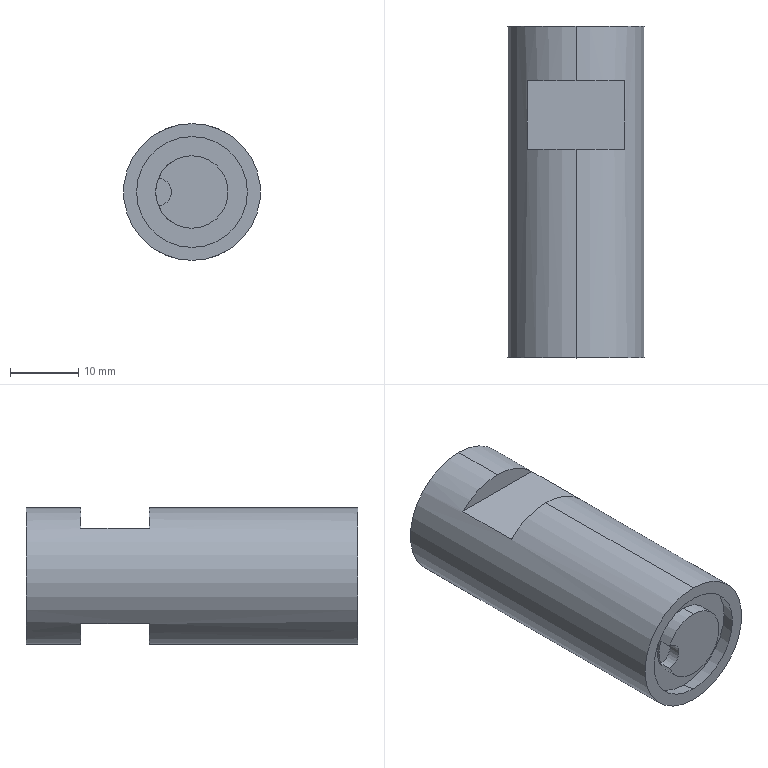Part | STEP file | OP10-151_seal rod (L) | 1 solid | 22 faces | box 20 x 48.5 x 20 mm | volume 14002 mm3 | plane 11 | cylinder 7 | cone 4 | commonest cylinder face diameters 5 x2 10.6 x2 20 x2 4 x1
STEP:
#1=CARTESIAN_POINT('',(0.,0.,0.));
#2=DIRECTION('',(0.,0.,1.));
#3=DIRECTION('',(1.,0.,0.));
#4=AXIS2_PLACEMENT_3D('',#1,#2,#3);
#5=CARTESIAN_POINT('',(0.,30.5,2.5));
#6=VERTEX_POINT('',#5);
#7=CARTESIAN_POINT('',(0.,48.5,2.5));
#8=VERTEX_POINT('',#7);
#9=CARTESIAN_POINT('',(0.,48.5,2.5));
#10=DIRECTION('',(0.,1.,0.));
#11=VECTOR('',#10,1.);
#12=LINE('',#9,#11);
#13=CARTESIAN_POINT('',(0.,48.5,0.));
#14=DIRECTION('',(0.,1.,0.));
#15=DIRECTION('',(0.,0.,1.));
#16=AXIS2_PLACEMENT_3D('',#13,#14,#15);
#17=CYLINDRICAL_SURFACE('',#16,2.5);
#18=CARTESIAN_POINT('',(6.283,0.));
#19=DIRECTION('',(0.,1.));
#20=VECTOR('',#19,1.);
#21=LINE('',#18,#20);
#22=(GEOMETRIC_REPRESENTATION_CONTEXT(2)PARAMETRIC_REPRESENTATION_CONTEXT()REPRESENTATION_CONTEXT('',''));
#23=DEFINITIONAL_REPRESENTATION('',(#21),#22);
#24=PCURVE('',#17,#23);
#25=CARTESIAN_POINT('',(0.,48.5,0.));
#26=DIRECTION('',(0.,1.,0.));
#27=DIRECTION('',(0.,0.,1.));
#28=AXIS2_PLACEMENT_3D('',#25,#26,#27);
#29=CYLINDRICAL_SURFACE('',#28,2.5);
#30=CARTESIAN_POINT('',(0.,0.));
#31=DIRECTION('',(0.,1.));
#32=VECTOR('',#31,1.);
#33=LINE('',#30,#32);
#34=(GEOMETRIC_REPRESENTATION_CONTEXT(2)PARAMETRIC_REPRESENTATION_CONTEXT()REPRESENTATION_CONTEXT('',''));
#35=DEFINITIONAL_REPRESENTATION('',(#33),#34);
#36=PCURVE('',#29,#35);
#37=SURFACE_CURVE('',#12,(#24,#36),.PCURVE_S1.);
#38=EDGE_CURVE('',#6,#8,#37,.T.);
#39=ORIENTED_EDGE('',*,*,#38,.T.);
#40=CARTESIAN_POINT('',(0.,48.5,-2.5));
#41=VERTEX_POINT('',#40);
#42=CARTESIAN_POINT('',(0.,48.5,0.));
#43=DIRECTION('',(0.,1.,0.));
#44=DIRECTION('',(0.,0.,1.));
#45=AXIS2_PLACEMENT_3D('',#42,#43,#44);
#46=CIRCLE('',#45,2.5);
#47=CARTESIAN_POINT('',(0.,0.));
#48=DIRECTION('',(1.,0.));
#49=VECTOR('',#48,1.);
#50=LINE('',#47,#49);
#51=(GEOMETRIC_REPRESENTATION_CONTEXT(2)PARAMETRIC_REPRESENTATION_CONTEXT()REPRESENTATION_CONTEXT('',''));
#52=DEFINITIONAL_REPRESENTATION('',(#50),#51);
#53=PCURVE('',#17,#52);
#54=CARTESIAN_POINT('',(0.,48.5,0.));
#55=DIRECTION('',(0.,1.,0.));
#56=DIRECTION('',(0.,0.,1.));
#57=AXIS2_PLACEMENT_3D('',#54,#55,#56);
#58=PLANE('',#57);
#59=CARTESIAN_POINT('',(0.,0.));
#60=DIRECTION('',(1.,0.));
#61=AXIS2_PLACEMENT_2D('',#59,#60);
#62=CIRCLE('',#61,2.5);
#63=(GEOMETRIC_REPRESENTATION_CONTEXT(2)PARAMETRIC_REPRESENTATION_CONTEXT()REPRESENTATION_CONTEXT('',''));
#64=DEFINITIONAL_REPRESENTATION('',(#62),#63);
#65=PCURVE('',#58,#64);
#66=SURFACE_CURVE('',#46,(#53,#65),.PCURVE_S1.);
#67=EDGE_CURVE('',#41,#8,#66,.T.);
#68=ORIENTED_EDGE('',*,*,#67,.F.);
#69=CARTESIAN_POINT('',(0.,30.5,-2.5));
#70=VERTEX_POINT('',#69);
#71=CARTESIAN_POINT('',(0.,48.5,-2.5));
#72=DIRECTION('',(0.,1.,0.));
#73=VECTOR('',#72,1.);
#74=LINE('',#71,#73);
#75=CARTESIAN_POINT('',(3.142,0.));
#76=DIRECTION('',(0.,1.));
#77=VECTOR('',#76,1.);
#78=LINE('',#75,#77);
#79=(GEOMETRIC_REPRESENTATION_CONTEXT(2)PARAMETRIC_REPRESENTATION_CONTEXT()REPRESENTATION_CONTEXT('',''));
#80=DEFINITIONAL_REPRESENTATION('',(#78),#79);
#81=PCURVE('',#17,#80);
#82=CARTESIAN_POINT('',(3.142,0.));
#83=DIRECTION('',(0.,1.));
#84=VECTOR('',#83,1.);
#85=LINE('',#82,#84);
#86=(GEOMETRIC_REPRESENTATION_CONTEXT(2)PARAMETRIC_REPRESENTATION_CONTEXT()REPRESENTATION_CONTEXT('',''));
#87=DEFINITIONAL_REPRESENTATION('',(#85),#86);
#88=PCURVE('',#29,#87);
#89=SURFACE_CURVE('',#74,(#81,#88),.PCURVE_S1.);
#90=EDGE_CURVE('',#70,#41,#89,.T.);
#91=ORIENTED_EDGE('',*,*,#90,.F.);
#92=CARTESIAN_POINT('',(0.,30.5,0.));
#93=DIRECTION('',(0.,1.,0.));
#94=DIRECTION('',(0.,0.,1.));
#95=AXIS2_PLACEMENT_3D('',#92,#93,#94);
#96=CIRCLE('',#95,2.5);
#97=CARTESIAN_POINT('',(0.,-18.));
#98=DIRECTION('',(1.,0.));
#99=VECTOR('',#98,1.);
#100=LINE('',#97,#99);
#101=(GEOMETRIC_REPRESENTATION_CONTEXT(2)PARAMETRIC_REPRESENTATION_CONTEXT()REPRESENTATION_CONTEXT('',''));
#102=DEFINITIONAL_REPRESENTATION('',(#100),#101);
#103=PCURVE('',#17,#102);
#104=CARTESIAN_POINT('',(0.,30.5,0.));
#105=DIRECTION('',(0.,1.,0.));
#106=DIRECTION('',(0.,0.,1.));
#107=AXIS2_PLACEMENT_3D('',#104,#105,#106);
#108=CONICAL_SURFACE('',#107,2.5,1.03);
#109=CARTESIAN_POINT('',(0.,0.));
#110=DIRECTION('',(1.,0.));
#111=VECTOR('',#110,1.);
#112=LINE('',#109,#111);
#113=(GEOMETRIC_REPRESENTATION_CONTEXT(2)PARAMETRIC_REPRESENTATION_CONTEXT()REPRESENTATION_CONTEXT('',''));
#114=DEFINITIONAL_REPRESENTATION('',(#112),#113);
#115=PCURVE('',#108,#114);
#116=SURFACE_CURVE('',#96,(#103,#115),.PCURVE_S1.);
#117=EDGE_CURVE('',#70,#6,#116,.T.);
#118=ORIENTED_EDGE('',*,*,#117,.T.);
#119=EDGE_LOOP('',(#39,#68,#91,#118));
#120=FACE_BOUND('',#119,.F.);
#121=ADVANCED_FACE('',(#120),#17,.F.);
#122=ORIENTED_EDGE('',*,*,#117,.F.);
#123=CARTESIAN_POINT('',(0.,28.998,0.));
#124=VERTEX_POINT('',#123);
#125=CARTESIAN_POINT('',(0.,30.5,-2.5));
#126=DIRECTION('',(0.,0.515,-0.8572));
#127=VECTOR('',#126,1.);
#128=LINE('',#125,#127);
#129=CARTESIAN_POINT('',(3.142,0.));
#130=DIRECTION('',(0.,1.));
#131=VECTOR('',#130,1.);
#132=LINE('',#129,#131);
#133=(GEOMETRIC_REPRESENTATION_CONTEXT(2)PARAMETRIC_REPRESENTATION_CONTEXT()REPRESENTATION_CONTEXT('',''));
#134=DEFINITIONAL_REPRESENTATION('',(#132),#133);
#135=PCURVE('',#108,#134);
#136=CARTESIAN_POINT('',(0.,30.5,0.));
#137=DIRECTION('',(0.,1.,0.));
#138=DIRECTION('',(0.,0.,1.));
#139=AXIS2_PLACEMENT_3D('',#136,#137,#138);
#140=CONICAL_SURFACE('',#139,2.5,1.03);
#141=CARTESIAN_POINT('',(3.142,0.));
#142=DIRECTION('',(0.,1.));
#143=VECTOR('',#142,1.);
#144=LINE('',#141,#143);
#145=(GEOMETRIC_REPRESENTATION_CONTEXT(2)PARAMETRIC_REPRESENTATION_CONTEXT()REPRESENTATION_CONTEXT('',''));
#146=DEFINITIONAL_REPRESENTATION('',(#144),#145);
#147=PCURVE('',#140,#146);
#148=SURFACE_CURVE('',#128,(#135,#147),.PCURVE_S1.);
#149=EDGE_CURVE('',#124,#70,#148,.T.);
#150=ORIENTED_EDGE('',*,*,#149,.F.);
#151=CARTESIAN_POINT('',(0.,30.5,2.5));
#152=DIRECTION('',(0.,0.515,0.8572));
#153=VECTOR('',#152,1.);
#154=LINE('',#151,#153);
#155=CARTESIAN_POINT('',(6.283,0.));
#156=DIRECTION('',(0.,1.));
#157=VECTOR('',#156,1.);
#158=LINE('',#155,#157);
#159=(GEOMETRIC_REPRESENTATION_CONTEXT(2)PARAMETRIC_REPRESENTATION_CONTEXT()REPRESENTATION_CONTEXT('',''));
#160=DEFINITIONAL_REPRESENTATION('',(#158),#159);
#161=PCURVE('',#108,#160);
#162=CARTESIAN_POINT('',(0.,0.));
#163=DIRECTION('',(0.,1.));
#164=VECTOR('',#163,1.);
#165=LINE('',#162,#164);
#166=(GEOMETRIC_REPRESENTATION_CONTEXT(2)PARAMETRIC_REPRESENTATION_CONTEXT()REPRESENTATION_CONTEXT('',''));
#167=DEFINITIONAL_REPRESENTATION('',(#165),#166);
#168=PCURVE('',#140,#167);
#169=SURFACE_CURVE('',#154,(#161,#168),.PCURVE_S1.);
#170=EDGE_CURVE('',#124,#6,#169,.T.);
#171=ORIENTED_EDGE('',*,*,#170,.T.);
#172=EDGE_LOOP('',(#122,#150,#171));
#173=FACE_BOUND('',#172,.F.);
#174=ADVANCED_FACE('',(#173),#108,.F.);
#175=CARTESIAN_POINT('',(0.,2.1,-5.3));
#176=VERTEX_POINT('',#175);
#177=CARTESIAN_POINT('',(0.,2.1,5.3));
#178=VERTEX_POINT('',#177);
#179=CARTESIAN_POINT('',(0.,2.1,0.));
#180=DIRECTION('',(0.,-1.,0.));
#181=DIRECTION('',(0.,0.,-1.));
#182=AXIS2_PLACEMENT_3D('',#179,#180,#181);
#183=CIRCLE('',#182,5.3);
#184=CARTESIAN_POINT('',(0.,2.1,0.));
#185=DIRECTION('',(0.,-1.,0.));
#186=DIRECTION('',(0.,0.,-1.));
#187=AXIS2_PLACEMENT_3D('',#184,#185,#186);
#188=CYLINDRICAL_SURFACE('',#187,5.3);
#189=CARTESIAN_POINT('',(0.,0.));
#190=DIRECTION('',(1.,0.));
#191=VECTOR('',#190,1.);
#192=LINE('',#189,#191);
#193=(GEOMETRIC_REPRESENTATION_CONTEXT(2)PARAMETRIC_REPRESENTATION_CONTEXT()REPRESENTATION_CONTEXT('',''));
#194=DEFINITIONAL_REPRESENTATION('',(#192),#193);
#195=PCURVE('',#188,#194);
#196=CARTESIAN_POINT('',(0.,2.1,0.));
#197=DIRECTION('',(0.,-1.,0.));
#198=DIRECTION('',(0.,0.,-1.));
#199=AXIS2_PLACEMENT_3D('',#196,#197,#198);
#200=PLANE('',#199);
#201=CARTESIAN_POINT('',(0.,0.));
#202=DIRECTION('',(1.,0.));
#203=AXIS2_PLACEMENT_2D('',#201,#202);
#204=CIRCLE('',#203,5.3);
#205=(GEOMETRIC_REPRESENTATION_CONTEXT(2)PARAMETRIC_REPRESENTATION_CONTEXT()REPRESENTATION_CONTEXT('',''));
#206=DEFINITIONAL_REPRESENTATION('',(#204),#205);
#207=PCURVE('',#200,#206);
#208=SURFACE_CURVE('',#183,(#195,#207),.PCURVE_S1.);
#209=EDGE_CURVE('',#176,#178,#208,.T.);
#210=ORIENTED_EDGE('',*,*,#209,.T.);
#211=CARTESIAN_POINT('',(0.,0.,5.3));
#212=VERTEX_POINT('',#211);
#213=CARTESIAN_POINT('',(0.,2.1,5.3));
#214=DIRECTION('',(0.,-1.,0.));
#215=VECTOR('',#214,1.);
#216=LINE('',#213,#215);
#217=CARTESIAN_POINT('',(3.142,0.));
#218=DIRECTION('',(0.,1.));
#219=VECTOR('',#218,1.);
#220=LINE('',#217,#219);
#221=(GEOMETRIC_REPRESENTATION_CONTEXT(2)PARAMETRIC_REPRESENTATION_CONTEXT()REPRESENTATION_CONTEXT('',''));
#222=DEFINITIONAL_REPRESENTATION('',(#220),#221);
#223=PCURVE('',#188,#222);
#224=CARTESIAN_POINT('',(0.,2.1,0.));
#225=DIRECTION('',(0.,-1.,0.));
#226=DIRECTION('',(0.,0.,-1.));
#227=AXIS2_PLACEMENT_3D('',#224,#225,#226);
#228=CYLINDRICAL_SURFACE('',#227,5.3);
#229=CARTESIAN_POINT('',(3.142,0.));
#230=DIRECTION('',(0.,1.));
#231=VECTOR('',#230,1.);
#232=LINE('',#229,#231);
#233=(GEOMETRIC_REPRESENTATION_CONTEXT(2)PARAMETRIC_REPRESENTATION_CONTEXT()REPRESENTATION_CONTEXT('',''));
#234=DEFINITIONAL_REPRESENTATION('',(#232),#233);
#235=PCURVE('',#228,#234);
#236=SURFACE_CURVE('',#216,(#223,#235),.PCURVE_S1.);
#237=EDGE_CURVE('',#178,#212,#236,.T.);
#238=ORIENTED_EDGE('',*,*,#237,.T.);
#239=CARTESIAN_POINT('',(0.,0.,-5.3));
#240=VERTEX_POINT('',#239);
#241=CARTESIAN_POINT('',(0.,0.,0.));
#242=DIRECTION('',(0.,-1.,0.));
#243=DIRECTION('',(0.,0.,-1.));
#244=AXIS2_PLACEMENT_3D('',#241,#242,#243);
#245=CIRCLE('',#244,5.3);
#246=CARTESIAN_POINT('',(0.,2.1));
#247=DIRECTION('',(1.,0.));
#248=VECTOR('',#247,1.);
#249=LINE('',#246,#248);
#250=(GEOMETRIC_REPRESENTATION_CONTEXT(2)PARAMETRIC_REPRESENTATION_CONTEXT()REPRESENTATION_CONTEXT('',''));
#251=DEFINITIONAL_REPRESENTATION('',(#249),#250);
#252=PCURVE('',#188,#251);
#253=CARTESIAN_POINT('',(0.,0.,0.));
#254=DIRECTION('',(0.,1.,0.));
#255=DIRECTION('',(0.,0.,1.));
#256=AXIS2_PLACEMENT_3D('',#253,#254,#255);
#257=PLANE('',#256);
#258=CARTESIAN_POINT('',(-5.3,0.));
#259=CARTESIAN_POINT('',(-5.3,9.18));
#260=CARTESIAN_POINT('',(2.65,4.59));
#261=CARTESIAN_POINT('',(10.6,0.));
#262=CARTESIAN_POINT('',(2.65,-4.59));
#263=CARTESIAN_POINT('',(-5.3,-9.18));
#264=CARTESIAN_POINT('',(-5.3,0.));
#265=(BOUNDED_CURVE()B_SPLINE_CURVE(2,(#258,#259,#260,#261,#262,#263,#264),.UNSPECIFIED.,.T.,.F.)B_SPLINE_CURVE_WITH_KNOTS((1,2,2,2,2,1),(-2.094,0.,2.094,4.189,6.283,8.378),.UNSPECIFIED.)CURVE()GEOMETRIC_REPRESENTATION_ITEM()RATIONAL_B_SPLINE_CURVE((1.,0.5,1.,0.5,1.,0.5,1.))REPRESENTATION_ITEM(''));
#266=(GEOMETRIC_REPRESENTATION_CONTEXT(2)PARAMETRIC_REPRESENTATION_CONTEXT()REPRESENTATION_CONTEXT('',''));
#267=DEFINITIONAL_REPRESENTATION('',(#265),#266);
#268=PCURVE('',#257,#267);
#269=SURFACE_CURVE('',#245,(#252,#268),.PCURVE_S1.);
#270=EDGE_CURVE('',#240,#212,#269,.T.);
#271=ORIENTED_EDGE('',*,*,#270,.F.);
#272=CARTESIAN_POINT('',(0.,2.1,-5.3));
#273=DIRECTION('',(0.,-1.,0.));
#274=VECTOR('',#273,1.);
#275=LINE('',#272,#274);
#276=CARTESIAN_POINT('',(0.,0.));
#277=DIRECTION('',(0.,1.));
#278=VECTOR('',#277,1.);
#279=LINE('',#276,#278);
#280=(GEOMETRIC_REPRESENTATION_CONTEXT(2)PARAMETRIC_REPRESENTATION_CONTEXT()REPRESENTATION_CONTEXT('',''));
#281=DEFINITIONAL_REPRESENTATION('',(#279),#280);
#282=PCURVE('',#188,#281);
#283=CARTESIAN_POINT('',(6.283,0.));
#284=DIRECTION('',(0.,1.));
#285=VECTOR('',#284,1.);
#286=LINE('',#283,#285);
#287=(GEOMETRIC_REPRESENTATION_CONTEXT(2)PARAMETRIC_REPRESENTATION_CONTEXT()REPRESENTATION_CONTEXT('',''));
#288=DEFINITIONAL_REPRESENTATION('',(#286),#287);
#289=PCURVE('',#228,#288);
#290=SURFACE_CURVE('',#275,(#282,#289),.PCURVE_S1.);
#291=EDGE_CURVE('',#176,#240,#290,.T.);
#292=ORIENTED_EDGE('',*,*,#291,.F.);
#293=EDGE_LOOP('',(#210,#238,#271,#292));
#294=FACE_BOUND('',#293,.T.);
#295=ADVANCED_FACE('',(#294),#188,.T.);
#296=CARTESIAN_POINT('',(0.,0.,-8.1));
#297=VERTEX_POINT('',#296);
#298=CARTESIAN_POINT('',(0.,2.1,-8.47));
#299=VERTEX_POINT('',#298);
#300=CARTESIAN_POINT('',(0.,0.,-8.1));
#301=DIRECTION('',(0.,0.9848,-0.1736));
#302=VECTOR('',#301,1.);
#303=LINE('',#300,#302);
#304=CARTESIAN_POINT('',(0.,0.,0.));
#305=DIRECTION('',(0.,1.,0.));
#306=DIRECTION('',(0.,0.,-1.));
#307=AXIS2_PLACEMENT_3D('',#304,#305,#306);
#308=CONICAL_SURFACE('',#307,8.1,0.1745);
#309=CARTESIAN_POINT('',(6.283,0.));
#310=DIRECTION('',(0.,1.));
#311=VECTOR('',#310,1.);
#312=LINE('',#309,#311);
#313=(GEOMETRIC_REPRESENTATION_CONTEXT(2)PARAMETRIC_REPRESENTATION_CONTEXT()REPRESENTATION_CONTEXT('',''));
#314=DEFINITIONAL_REPRESENTATION('',(#312),#313);
#315=PCURVE('',#308,#314);
#316=CARTESIAN_POINT('',(0.,0.,0.));
#317=DIRECTION('',(0.,1.,0.));
#318=DIRECTION('',(0.,0.,-1.));
#319=AXIS2_PLACEMENT_3D('',#316,#317,#318);
#320=CONICAL_SURFACE('',#319,8.1,0.1745);
#321=CARTESIAN_POINT('',(0.,0.));
#322=DIRECTION('',(0.,1.));
#323=VECTOR('',#322,1.);
#324=LINE('',#321,#323);
#325=(GEOMETRIC_REPRESENTATION_CONTEXT(2)PARAMETRIC_REPRESENTATION_CONTEXT()REPRESENTATION_CONTEXT('',''));
#326=DEFINITIONAL_REPRESENTATION('',(#324),#325);
#327=PCURVE('',#320,#326);
#328=SURFACE_CURVE('',#303,(#315,#327),.PCURVE_S1.);
#329=EDGE_CURVE('',#297,#299,#328,.T.);
#330=ORIENTED_EDGE('',*,*,#329,.T.);
#331=CARTESIAN_POINT('',(0.,2.1,8.47));
#332=VERTEX_POINT('',#331);
#333=CARTESIAN_POINT('',(0.,2.1,0.));
#334=DIRECTION('',(0.,-1.,0.));
#335=DIRECTION('',(0.,0.,-1.));
#336=AXIS2_PLACEMENT_3D('',#333,#334,#335);
#337=CIRCLE('',#336,8.47);
#338=CARTESIAN_POINT('',(6.283,2.1));
#339=DIRECTION('',(-1.,0.));
#340=VECTOR('',#339,1.);
#341=LINE('',#338,#340);
#342=(GEOMETRIC_REPRESENTATION_CONTEXT(2)PARAMETRIC_REPRESENTATION_CONTEXT()REPRESENTATION_CONTEXT('',''));
#343=DEFINITIONAL_REPRESENTATION('',(#341),#342);
#344=PCURVE('',#308,#343);
#345=CARTESIAN_POINT('',(0.,0.));
#346=DIRECTION('',(1.,0.));
#347=AXIS2_PLACEMENT_2D('',#345,#346);
#348=CIRCLE('',#347,8.47);
#349=(GEOMETRIC_REPRESENTATION_CONTEXT(2)PARAMETRIC_REPRESENTATION_CONTEXT()REPRESENTATION_CONTEXT('',''));
#350=DEFINITIONAL_REPRESENTATION('',(#348),#349);
#351=PCURVE('',#200,#350);
#352=SURFACE_CURVE('',#337,(#344,#351),.PCURVE_S1.);
#353=EDGE_CURVE('',#299,#332,#352,.T.);
#354=ORIENTED_EDGE('',*,*,#353,.T.);
#355=CARTESIAN_POINT('',(0.,0.,8.1));
#356=VERTEX_POINT('',#355);
#357=CARTESIAN_POINT('',(0.,0.,8.1));
#358=DIRECTION('',(0.,0.9848,0.1736));
#359=VECTOR('',#358,1.);
#360=LINE('',#357,#359);
#361=CARTESIAN_POINT('',(3.142,0.));
#362=DIRECTION('',(0.,1.));
#363=VECTOR('',#362,1.);
#364=LINE('',#361,#363);
#365=(GEOMETRIC_REPRESENTATION_CONTEXT(2)PARAMETRIC_REPRESENTATION_CONTEXT()REPRESENTATION_CONTEXT('',''));
#366=DEFINITIONAL_REPRESENTATION('',(#364),#365);
#367=PCURVE('',#308,#366);
#368=CARTESIAN_POINT('',(3.142,0.));
#369=DIRECTION('',(0.,1.));
#370=VECTOR('',#369,1.);
#371=LINE('',#368,#370);
#372=(GEOMETRIC_REPRESENTATION_CONTEXT(2)PARAMETRIC_REPRESENTATION_CONTEXT()REPRESENTATION_CONTEXT('',''));
#373=DEFINITIONAL_REPRESENTATION('',(#371),#372);
#374=PCURVE('',#320,#373);
#375=SURFACE_CURVE('',#360,(#367,#374),.PCURVE_S1.);
#376=EDGE_CURVE('',#356,#332,#375,.T.);
#377=ORIENTED_EDGE('',*,*,#376,.F.);
#378=CARTESIAN_POINT('',(0.,0.,0.));
#379=DIRECTION('',(0.,-1.,0.));
#380=DIRECTION('',(0.,0.,-1.));
#381=AXIS2_PLACEMENT_3D('',#378,#379,#380);
#382=CIRCLE('',#381,8.1);
#383=CARTESIAN_POINT('',(6.283,0.));
#384=DIRECTION('',(-1.,0.));
#385=VECTOR('',#384,1.);
#386=LINE('',#383,#385);
#387=(GEOMETRIC_REPRESENTATION_CONTEXT(2)PARAMETRIC_REPRESENTATION_CONTEXT()REPRESENTATION_CONTEXT('',''));
#388=DEFINITIONAL_REPRESENTATION('',(#386),#387);
#389=PCURVE('',#308,#388);
#390=CARTESIAN_POINT('',(0.,0.,0.));
#391=DIRECTION('',(0.,1.,0.));
#392=DIRECTION('',(0.,0.,1.));
#393=AXIS2_PLACEMENT_3D('',#390,#391,#392);
#394=PLANE('',#393);
#395=CARTESIAN_POINT('',(-8.1,0.));
#396=CARTESIAN_POINT('',(-8.1,14.03));
#397=CARTESIAN_POINT('',(4.05,7.015));
#398=CARTESIAN_POINT('',(16.2,0.));
#399=CARTESIAN_POINT('',(4.05,-7.015));
#400=CARTESIAN_POINT('',(-8.1,-14.03));
#401=CARTESIAN_POINT('',(-8.1,0.));
#402=(BOUNDED_CURVE()B_SPLINE_CURVE(2,(#395,#396,#397,#398,#399,#400,#401),.UNSPECIFIED.,.T.,.F.)B_SPLINE_CURVE_WITH_KNOTS((1,2,2,2,2,1),(-2.094,0.,2.094,4.189,6.283,8.378),.UNSPECIFIED.)CURVE()GEOMETRIC_REPRESENTATION_ITEM()RATIONAL_B_SPLINE_CURVE((1.,0.5,1.,0.5,1.,0.5,1.))REPRESENTATION_ITEM(''));
#403=(GEOMETRIC_REPRESENTATION_CONTEXT(2)PARAMETRIC_REPRESENTATION_CONTEXT()REPRESENTATION_CONTEXT('',''));
#404=DEFINITIONAL_REPRESENTATION('',(#402),#403);
#405=PCURVE('',#394,#404);
#406=SURFACE_CURVE('',#382,(#389,#405),.PCURVE_S1.);
#407=EDGE_CURVE('',#297,#356,#406,.T.);
#408=ORIENTED_EDGE('',*,*,#407,.F.);
#409=EDGE_LOOP('',(#330,#354,#377,#408));
#410=FACE_BOUND('',#409,.F.);
#411=ADVANCED_FACE('',(#410),#308,.F.);
#412=CARTESIAN_POINT('',(0.,48.5,10.));
#413=VERTEX_POINT('',#412);
#414=CARTESIAN_POINT('',(0.,48.5,-10.));
#415=VERTEX_POINT('',#414);
#416=CARTESIAN_POINT('',(0.,48.5,0.));
#417=DIRECTION('',(0.,1.,0.));
#418=DIRECTION('',(0.,0.,1.));
#419=AXIS2_PLACEMENT_3D('',#416,#417,#418);
#420=CIRCLE('',#419,10.);
#421=CARTESIAN_POINT('',(0.,48.5,0.));
#422=DIRECTION('',(0.,-1.,0.));
#423=DIRECTION('',(0.,0.,-1.));
#424=AXIS2_PLACEMENT_3D('',#421,#422,#423);
#425=CYLINDRICAL_SURFACE('',#424,10.);
#426=CARTESIAN_POINT('',(3.142,0.));
#427=DIRECTION('',(-1.,0.));
#428=VECTOR('',#427,1.);
#429=LINE('',#426,#428);
#430=(GEOMETRIC_REPRESENTATION_CONTEXT(2)PARAMETRIC_REPRESENTATION_CONTEXT()REPRESENTATION_CONTEXT('',''));
#431=DEFINITIONAL_REPRESENTATION('',(#429),#430);
#432=PCURVE('',#425,#431);
#433=CARTESIAN_POINT('',(0.,0.));
#434=DIRECTION('',(1.,0.));
#435=AXIS2_PLACEMENT_2D('',#433,#434);
#436=CIRCLE('',#435,10.);
#437=(GEOMETRIC_REPRESENTATION_CONTEXT(2)PARAMETRIC_REPRESENTATION_CONTEXT()REPRESENTATION_CONTEXT('',''));
#438=DEFINITIONAL_REPRESENTATION('',(#436),#437);
#439=PCURVE('',#58,#438);
#440=SURFACE_CURVE('',#420,(#432,#439),.PCURVE_S1.);
#441=EDGE_CURVE('',#413,#415,#440,.T.);
#442=ORIENTED_EDGE('',*,*,#441,.F.);
#443=CARTESIAN_POINT('',(0.,40.5,10.));
#444=VERTEX_POINT('',#443);
#445=CARTESIAN_POINT('',(0.,48.5,10.));
#446=DIRECTION('',(0.,-1.,0.));
#447=VECTOR('',#446,1.);
#448=LINE('',#445,#447);
#449=CARTESIAN_POINT('',(3.142,0.));
#450=DIRECTION('',(0.,1.));
#451=VECTOR('',#450,1.);
#452=LINE('',#449,#451);
#453=(GEOMETRIC_REPRESENTATION_CONTEXT(2)PARAMETRIC_REPRESENTATION_CONTEXT()REPRESENTATION_CONTEXT('',''));
#454=DEFINITIONAL_REPRESENTATION('',(#452),#453);
#455=PCURVE('',#425,#454);
#456=CARTESIAN_POINT('',(0.,48.5,0.));
#457=DIRECTION('',(0.,-1.,0.));
#458=DIRECTION('',(0.,0.,-1.));
#459=AXIS2_PLACEMENT_3D('',#456,#457,#458);
#460=CYLINDRICAL_SURFACE('',#459,10.);
#461=CARTESIAN_POINT('',(3.142,0.));
#462=DIRECTION('',(0.,1.));
#463=VECTOR('',#462,1.);
#464=LINE('',#461,#463);
#465=(GEOMETRIC_REPRESENTATION_CONTEXT(2)PARAMETRIC_REPRESENTATION_CONTEXT()REPRESENTATION_CONTEXT('',''));
#466=DEFINITIONAL_REPRESENTATION('',(#464),#465);
#467=PCURVE('',#460,#466);
#468=SURFACE_CURVE('',#448,(#455,#467),.PCURVE_S1.);
#469=EDGE_CURVE('',#413,#444,#468,.T.);
#470=ORIENTED_EDGE('',*,*,#469,.T.);
#471=CARTESIAN_POINT('',(7.141,40.5,7.));
#472=VERTEX_POINT('',#471);
#473=CARTESIAN_POINT('',(0.,40.5,0.));
#474=DIRECTION('',(0.,-1.,0.));
#475=DIRECTION('',(0.,0.,-1.));
#476=AXIS2_PLACEMENT_3D('',#473,#474,#475);
#477=CIRCLE('',#476,10.);
#478=CARTESIAN_POINT('',(0.,8.));
#479=DIRECTION('',(1.,0.));
#480=VECTOR('',#479,1.);
#481=LINE('',#478,#480);
#482=(GEOMETRIC_REPRESENTATION_CONTEXT(2)PARAMETRIC_REPRESENTATION_CONTEXT()REPRESENTATION_CONTEXT('',''));
#483=DEFINITIONAL_REPRESENTATION('',(#481),#482);
#484=PCURVE('',#425,#483);
#485=CARTESIAN_POINT('',(-16.827,40.5,55.5));
#486=DIRECTION('',(0.,-1.,0.));
#487=DIRECTION('',(0.,0.,-1.));
#488=AXIS2_PLACEMENT_3D('',#485,#486,#487);
#489=PLANE('',#488);
#490=CARTESIAN_POINT('',(55.5,16.827));
#491=DIRECTION('',(1.,0.));
#492=AXIS2_PLACEMENT_2D('',#490,#491);
#493=CIRCLE('',#492,10.);
#494=(GEOMETRIC_REPRESENTATION_CONTEXT(2)PARAMETRIC_REPRESENTATION_CONTEXT()REPRESENTATION_CONTEXT('',''));
#495=DEFINITIONAL_REPRESENTATION('',(#493),#494);
#496=PCURVE('',#489,#495);
#497=SURFACE_CURVE('',#477,(#484,#496),.PCURVE_S1.);
#498=EDGE_CURVE('',#472,#444,#497,.T.);
#499=ORIENTED_EDGE('',*,*,#498,.F.);
#500=CARTESIAN_POINT('',(7.141,30.5,7.));
#501=VERTEX_POINT('',#500);
#502=CARTESIAN_POINT('',(7.141,48.5,7.));
#503=DIRECTION('',(0.,-1.,0.));
#504=VECTOR('',#503,1.);
#505=LINE('',#502,#504);
#506=CARTESIAN_POINT('',(2.346,0.));
#507=DIRECTION('',(0.,1.));
#508=VECTOR('',#507,1.);
#509=LINE('',#506,#508);
#510=(GEOMETRIC_REPRESENTATION_CONTEXT(2)PARAMETRIC_REPRESENTATION_CONTEXT()REPRESENTATION_CONTEXT('',''));
#511=DEFINITIONAL_REPRESENTATION('',(#509),#510);
#512=PCURVE('',#425,#511);
#513=CARTESIAN_POINT('',(0.,0.,7.));
#514=DIRECTION('',(0.,0.,-1.));
#515=DIRECTION('',(1.,0.,0.));
#516=AXIS2_PLACEMENT_3D('',#513,#514,#515);
#517=PLANE('',#516);
#518=CARTESIAN_POINT('',(7.141,-48.5));
#519=DIRECTION('',(0.,1.));
#520=VECTOR('',#519,1.);
#521=LINE('',#518,#520);
#522=(GEOMETRIC_REPRESENTATION_CONTEXT(2)PARAMETRIC_REPRESENTATION_CONTEXT()REPRESENTATION_CONTEXT('',''));
#523=DEFINITIONAL_REPRESENTATION('',(#521),#522);
#524=PCURVE('',#517,#523);
#525=SURFACE_CURVE('',#505,(#512,#524),.PCURVE_S1.);
#526=EDGE_CURVE('',#472,#501,#525,.T.);
#527=ORIENTED_EDGE('',*,*,#526,.T.);
#528=CARTESIAN_POINT('',(0.,30.5,10.));
#529=VERTEX_POINT('',#528);
#530=CARTESIAN_POINT('',(0.,30.5,0.));
#531=DIRECTION('',(0.,1.,0.));
#532=DIRECTION('',(0.,0.,1.));
#533=AXIS2_PLACEMENT_3D('',#530,#531,#532);
#534=CIRCLE('',#533,10.);
#535=CARTESIAN_POINT('',(3.142,18.));
#536=DIRECTION('',(-1.,0.));
#537=VECTOR('',#536,1.);
#538=LINE('',#535,#537);
#539=(GEOMETRIC_REPRESENTATION_CONTEXT(2)PARAMETRIC_REPRESENTATION_CONTEXT()REPRESENTATION_CONTEXT('',''));
#540=DEFINITIONAL_REPRESENTATION('',(#538),#539);
#541=PCURVE('',#425,#540);
#542=CARTESIAN_POINT('',(-16.827,30.5,55.5));
#543=DIRECTION('',(0.,1.,0.));
#544=DIRECTION('',(0.,0.,1.));
#545=AXIS2_PLACEMENT_3D('',#542,#543,#544);
#546=PLANE('',#545);
#547=CARTESIAN_POINT('',(-55.5,16.827));
#548=DIRECTION('',(1.,0.));
#549=AXIS2_PLACEMENT_2D('',#547,#548);
#550=CIRCLE('',#549,10.);
#551=(GEOMETRIC_REPRESENTATION_CONTEXT(2)PARAMETRIC_REPRESENTATION_CONTEXT()REPRESENTATION_CONTEXT('',''));
#552=DEFINITIONAL_REPRESENTATION('',(#550),#551);
#553=PCURVE('',#546,#552);
#554=SURFACE_CURVE('',#534,(#541,#553),.PCURVE_S1.);
#555=EDGE_CURVE('',#529,#501,#554,.T.);
#556=ORIENTED_EDGE('',*,*,#555,.F.);
#557=CARTESIAN_POINT('',(0.,0.,10.));
#558=VERTEX_POINT('',#557);
#559=CARTESIAN_POINT('',(0.,48.5,10.));
#560=DIRECTION('',(0.,-1.,0.));
#561=VECTOR('',#560,1.);
#562=LINE('',#559,#561);
#563=CARTESIAN_POINT('',(3.142,0.));
#564=DIRECTION('',(0.,1.));
#565=VECTOR('',#564,1.);
#566=LINE('',#563,#565);
#567=(GEOMETRIC_REPRESENTATION_CONTEXT(2)PARAMETRIC_REPRESENTATION_CONTEXT()REPRESENTATION_CONTEXT('',''));
#568=DEFINITIONAL_REPRESENTATION('',(#566),#567);
#569=PCURVE('',#425,#568);
#570=CARTESIAN_POINT('',(3.142,0.));
#571=DIRECTION('',(0.,1.));
#572=VECTOR('',#571,1.);
#573=LINE('',#570,#572);
#574=(GEOMETRIC_REPRESENTATION_CONTEXT(2)PARAMETRIC_REPRESENTATION_CONTEXT()REPRESENTATION_CONTEXT('',''));
#575=DEFINITIONAL_REPRESENTATION('',(#573),#574);
#576=PCURVE('',#460,#575);
#577=SURFACE_CURVE('',#562,(#569,#576),.PCURVE_S1.);
#578=EDGE_CURVE('',#529,#558,#577,.T.);
#579=ORIENTED_EDGE('',*,*,#578,.T.);
#580=CARTESIAN_POINT('',(0.,0.,-10.));
#581=VERTEX_POINT('',#580);
#582=CARTESIAN_POINT('',(0.,0.,0.));
#583=DIRECTION('',(0.,1.,0.));
#584=DIRECTION('',(0.,0.,1.));
#585=AXIS2_PLACEMENT_3D('',#582,#583,#584);
#586=CIRCLE('',#585,10.);
#587=CARTESIAN_POINT('',(3.142,48.5));
#588=DIRECTION('',(-1.,0.));
#589=VECTOR('',#588,1.);
#590=LINE('',#587,#589);
#591=(GEOMETRIC_REPRESENTATION_CONTEXT(2)PARAMETRIC_REPRESENTATION_CONTEXT()REPRESENTATION_CONTEXT('',''));
#592=DEFINITIONAL_REPRESENTATION('',(#590),#591);
#593=PCURVE('',#425,#592);
#594=CARTESIAN_POINT('',(0.,0.));
#595=DIRECTION('',(1.,0.));
#596=AXIS2_PLACEMENT_2D('',#594,#595);
#597=CIRCLE('',#596,10.);
#598=(GEOMETRIC_REPRESENTATION_CONTEXT(2)PARAMETRIC_REPRESENTATION_CONTEXT()REPRESENTATION_CONTEXT('',''));
#599=DEFINITIONAL_REPRESENTATION('',(#597),#598);
#600=PCURVE('',#394,#599);
#601=SURFACE_CURVE('',#586,(#593,#600),.PCURVE_S1.);
#602=EDGE_CURVE('',#558,#581,#601,.T.);
#603=ORIENTED_EDGE('',*,*,#602,.T.);
#604=CARTESIAN_POINT('',(0.,30.5,-10.));
#605=VERTEX_POINT('',#604);
#606=CARTESIAN_POINT('',(0.,48.5,-10.));
#607=DIRECTION('',(0.,-1.,0.));
#608=VECTOR('',#607,1.);
#609=LINE('',#606,#608);
#610=CARTESIAN_POINT('',(0.,0.));
#611=DIRECTION('',(0.,1.));
#612=VECTOR('',#611,1.);
#613=LINE('',#610,#612);
#614=(GEOMETRIC_REPRESENTATION_CONTEXT(2)PARAMETRIC_REPRESENTATION_CONTEXT()REPRESENTATION_CONTEXT('',''));
#615=DEFINITIONAL_REPRESENTATION('',(#613),#614);
#616=PCURVE('',#425,#615);
#617=CARTESIAN_POINT('',(6.283,0.));
#618=DIRECTION('',(0.,1.));
#619=VECTOR('',#618,1.);
#620=LINE('',#617,#619);
#621=(GEOMETRIC_REPRESENTATION_CONTEXT(2)PARAMETRIC_REPRESENTATION_CONTEXT()REPRESENTATION_CONTEXT('',''));
#622=DEFINITIONAL_REPRESENTATION('',(#620),#621);
#623=PCURVE('',#460,#622);
#624=SURFACE_CURVE('',#609,(#616,#623),.PCURVE_S1.);
#625=EDGE_CURVE('',#605,#581,#624,.T.);
#626=ORIENTED_EDGE('',*,*,#625,.F.);
#627=CARTESIAN_POINT('',(7.141,30.5,-7.));
#628=VERTEX_POINT('',#627);
#629=CARTESIAN_POINT('',(0.,30.5,0.));
#630=DIRECTION('',(0.,-1.,0.));
#631=DIRECTION('',(0.,0.,-1.));
#632=AXIS2_PLACEMENT_3D('',#629,#630,#631);
#633=CIRCLE('',#632,10.);
#634=CARTESIAN_POINT('',(0.,18.));
#635=DIRECTION('',(1.,0.));
#636=VECTOR('',#635,1.);
#637=LINE('',#634,#636);
#638=(GEOMETRIC_REPRESENTATION_CONTEXT(2)PARAMETRIC_REPRESENTATION_CONTEXT()REPRESENTATION_CONTEXT('',''));
#639=DEFINITIONAL_REPRESENTATION('',(#637),#638);
#640=PCURVE('',#425,#639);
#641=CARTESIAN_POINT('',(-16.827,30.5,-55.5));
#642=DIRECTION('',(0.,-1.,0.));
#643=DIRECTION('',(0.,0.,-1.));
#644=AXIS2_PLACEMENT_3D('',#641,#642,#643);
#645=PLANE('',#644);
#646=CARTESIAN_POINT('',(-55.5,16.827));
#647=DIRECTION('',(1.,0.));
#648=AXIS2_PLACEMENT_2D('',#646,#647);
#649=CIRCLE('',#648,10.);
#650=(GEOMETRIC_REPRESENTATION_CONTEXT(2)PARAMETRIC_REPRESENTATION_CONTEXT()REPRESENTATION_CONTEXT('',''));
#651=DEFINITIONAL_REPRESENTATION('',(#649),#650);
#652=PCURVE('',#645,#651);
#653=SURFACE_CURVE('',#633,(#640,#652),.PCURVE_S1.);
#654=EDGE_CURVE('',#605,#628,#653,.T.);
#655=ORIENTED_EDGE('',*,*,#654,.T.);
#656=CARTESIAN_POINT('',(7.141,40.5,-7.));
#657=VERTEX_POINT('',#656);
#658=CARTESIAN_POINT('',(7.141,48.5,-7.));
#659=DIRECTION('',(0.,1.,0.));
#660=VECTOR('',#659,1.);
#661=LINE('',#658,#660);
#662=CARTESIAN_POINT('',(0.7954,0.));
#663=DIRECTION('',(0.,-1.));
#664=VECTOR('',#663,1.);
#665=LINE('',#662,#664);
#666=(GEOMETRIC_REPRESENTATION_CONTEXT(2)PARAMETRIC_REPRESENTATION_CONTEXT()REPRESENTATION_CONTEXT('',''));
#667=DEFINITIONAL_REPRESENTATION('',(#665),#666);
#668=PCURVE('',#425,#667);
#669=CARTESIAN_POINT('',(0.,0.,-7.));
#670=DIRECTION('',(0.,0.,1.));
#671=DIRECTION('',(1.,0.,0.));
#672=AXIS2_PLACEMENT_3D('',#669,#670,#671);
#673=PLANE('',#672);
#674=CARTESIAN_POINT('',(7.141,48.5));
#675=DIRECTION('',(0.,1.));
#676=VECTOR('',#675,1.);
#677=LINE('',#674,#676);
#678=(GEOMETRIC_REPRESENTATION_CONTEXT(2)PARAMETRIC_REPRESENTATION_CONTEXT()REPRESENTATION_CONTEXT('',''));
#679=DEFINITIONAL_REPRESENTATION('',(#677),#678);
#680=PCURVE('',#673,#679);
#681=SURFACE_CURVE('',#661,(#668,#680),.PCURVE_S1.);
#682=EDGE_CURVE('',#628,#657,#681,.T.);
#683=ORIENTED_EDGE('',*,*,#682,.T.);
#684=CARTESIAN_POINT('',(0.,40.5,-10.));
#685=VERTEX_POINT('',#684);
#686=CARTESIAN_POINT('',(0.,40.5,0.));
#687=DIRECTION('',(0.,1.,0.));
#688=DIRECTION('',(0.,0.,1.));
#689=AXIS2_PLACEMENT_3D('',#686,#687,#688);
#690=CIRCLE('',#689,10.);
#691=CARTESIAN_POINT('',(3.142,8.));
#692=DIRECTION('',(-1.,0.));
#693=VECTOR('',#692,1.);
#694=LINE('',#691,#693);
#695=(GEOMETRIC_REPRESENTATION_CONTEXT(2)PARAMETRIC_REPRESENTATION_CONTEXT()REPRESENTATION_CONTEXT('',''));
#696=DEFINITIONAL_REPRESENTATION('',(#694),#695);
#697=PCURVE('',#425,#696);
#698=CARTESIAN_POINT('',(-16.827,40.5,-55.5));
#699=DIRECTION('',(0.,1.,0.));
#700=DIRECTION('',(0.,0.,1.));
#701=AXIS2_PLACEMENT_3D('',#698,#699,#700);
#702=PLANE('',#701);
#703=CARTESIAN_POINT('',(55.5,16.827));
#704=DIRECTION('',(1.,0.));
#705=AXIS2_PLACEMENT_2D('',#703,#704);
#706=CIRCLE('',#705,10.);
#707=(GEOMETRIC_REPRESENTATION_CONTEXT(2)PARAMETRIC_REPRESENTATION_CONTEXT()REPRESENTATION_CONTEXT('',''));
#708=DEFINITIONAL_REPRESENTATION('',(#706),#707);
#709=PCURVE('',#702,#708);
#710=SURFACE_CURVE('',#690,(#697,#709),.PCURVE_S1.);
#711=EDGE_CURVE('',#657,#685,#710,.T.);
#712=ORIENTED_EDGE('',*,*,#711,.T.);
#713=CARTESIAN_POINT('',(0.,48.5,-10.));
#714=DIRECTION('',(0.,-1.,0.));
#715=VECTOR('',#714,1.);
#716=LINE('',#713,#715);
#717=CARTESIAN_POINT('',(0.,0.));
#718=DIRECTION('',(0.,1.));
#719=VECTOR('',#718,1.);
#720=LINE('',#717,#719);
#721=(GEOMETRIC_REPRESENTATION_CONTEXT(2)PARAMETRIC_REPRESENTATION_CONTEXT()REPRESENTATION_CONTEXT('',''));
#722=DEFINITIONAL_REPRESENTATION('',(#720),#721);
#723=PCURVE('',#425,#722);
#724=CARTESIAN_POINT('',(6.283,0.));
#725=DIRECTION('',(0.,1.));
#726=VECTOR('',#725,1.);
#727=LINE('',#724,#726);
#728=(GEOMETRIC_REPRESENTATION_CONTEXT(2)PARAMETRIC_REPRESENTATION_CONTEXT()REPRESENTATION_CONTEXT('',''));
#729=DEFINITIONAL_REPRESENTATION('',(#727),#728);
#730=PCURVE('',#460,#729);
#731=SURFACE_CURVE('',#716,(#723,#730),.PCURVE_S1.);
#732=EDGE_CURVE('',#415,#685,#731,.T.);
#733=ORIENTED_EDGE('',*,*,#732,.F.);
#734=EDGE_LOOP('',(#442,#470,#499,#527,#556,#579,#603,#626,#655,#683,#712,#733));
#735=FACE_BOUND('',#734,.T.);
#736=ADVANCED_FACE('',(#735),#425,.T.);
#737=ORIENTED_EDGE('',*,*,#469,.F.);
#738=CARTESIAN_POINT('',(0.,48.5,0.));
#739=DIRECTION('',(0.,1.,0.));
#740=DIRECTION('',(0.,0.,1.));
#741=AXIS2_PLACEMENT_3D('',#738,#739,#740);
#742=CIRCLE('',#741,10.);
#743=CARTESIAN_POINT('',(9.425,0.));
#744=DIRECTION('',(-1.,0.));
#745=VECTOR('',#744,1.);
#746=LINE('',#743,#745);
#747=(GEOMETRIC_REPRESENTATION_CONTEXT(2)PARAMETRIC_REPRESENTATION_CONTEXT()REPRESENTATION_CONTEXT('',''));
#748=DEFINITIONAL_REPRESENTATION('',(#746),#747);
#749=PCURVE('',#460,#748);
#750=CARTESIAN_POINT('',(0.,0.));
#751=DIRECTION('',(1.,0.));
#752=AXIS2_PLACEMENT_2D('',#750,#751);
#753=CIRCLE('',#752,10.);
#754=(GEOMETRIC_REPRESENTATION_CONTEXT(2)PARAMETRIC_REPRESENTATION_CONTEXT()REPRESENTATION_CONTEXT('',''));
#755=DEFINITIONAL_REPRESENTATION('',(#753),#754);
#756=PCURVE('',#58,#755);
#757=SURFACE_CURVE('',#742,(#749,#756),.PCURVE_S1.);
#758=EDGE_CURVE('',#415,#413,#757,.T.);
#759=ORIENTED_EDGE('',*,*,#758,.F.);
#760=ORIENTED_EDGE('',*,*,#732,.T.);
#761=CARTESIAN_POINT('',(-7.141,40.5,-7.));
#762=VERTEX_POINT('',#761);
#763=CARTESIAN_POINT('',(0.,40.5,0.));
#764=DIRECTION('',(0.,1.,0.));
#765=DIRECTION('',(0.,0.,1.));
#766=AXIS2_PLACEMENT_3D('',#763,#764,#765);
#767=CIRCLE('',#766,10.);
#768=CARTESIAN_POINT('',(9.425,8.));
#769=DIRECTION('',(-1.,0.));
#770=VECTOR('',#769,1.);
#771=LINE('',#768,#770);
#772=(GEOMETRIC_REPRESENTATION_CONTEXT(2)PARAMETRIC_REPRESENTATION_CONTEXT()REPRESENTATION_CONTEXT('',''));
#773=DEFINITIONAL_REPRESENTATION('',(#771),#772);
#774=PCURVE('',#460,#773);
#775=CARTESIAN_POINT('',(55.5,16.827));
#776=DIRECTION('',(1.,0.));
#777=AXIS2_PLACEMENT_2D('',#775,#776);
#778=CIRCLE('',#777,10.);
#779=(GEOMETRIC_REPRESENTATION_CONTEXT(2)PARAMETRIC_REPRESENTATION_CONTEXT()REPRESENTATION_CONTEXT('',''));
#780=DEFINITIONAL_REPRESENTATION('',(#778),#779);
#781=PCURVE('',#702,#780);
#782=SURFACE_CURVE('',#767,(#774,#781),.PCURVE_S1.);
#783=EDGE_CURVE('',#685,#762,#782,.T.);
#784=ORIENTED_EDGE('',*,*,#783,.T.);
#785=CARTESIAN_POINT('',(-7.141,30.5,-7.));
#786=VERTEX_POINT('',#785);
#787=CARTESIAN_POINT('',(-7.141,48.5,-7.));
#788=DIRECTION('',(0.,-1.,0.));
#789=VECTOR('',#788,1.);
#790=LINE('',#787,#789);
#791=CARTESIAN_POINT('',(5.488,0.));
#792=DIRECTION('',(0.,1.));
#793=VECTOR('',#792,1.);
#794=LINE('',#791,#793);
#795=(GEOMETRIC_REPRESENTATION_CONTEXT(2)PARAMETRIC_REPRESENTATION_CONTEXT()REPRESENTATION_CONTEXT('',''));
#796=DEFINITIONAL_REPRESENTATION('',(#794),#795);
#797=PCURVE('',#460,#796);
#798=CARTESIAN_POINT('',(-7.141,48.5));
#799=DIRECTION('',(0.,-1.));
#800=VECTOR('',#799,1.);
#801=LINE('',#798,#800);
#802=(GEOMETRIC_REPRESENTATION_CONTEXT(2)PARAMETRIC_REPRESENTATION_CONTEXT()REPRESENTATION_CONTEXT('',''));
#803=DEFINITIONAL_REPRESENTATION('',(#801),#802);
#804=PCURVE('',#673,#803);
#805=SURFACE_CURVE('',#790,(#797,#804),.PCURVE_S1.);
#806=EDGE_CURVE('',#762,#786,#805,.T.);
#807=ORIENTED_EDGE('',*,*,#806,.T.);
#808=CARTESIAN_POINT('',(0.,30.5,0.));
#809=DIRECTION('',(0.,-1.,0.));
#810=DIRECTION('',(0.,0.,-1.));
#811=AXIS2_PLACEMENT_3D('',#808,#809,#810);
#812=CIRCLE('',#811,10.);
#813=CARTESIAN_POINT('',(0.,18.));
#814=DIRECTION('',(1.,0.));
#815=VECTOR('',#814,1.);
#816=LINE('',#813,#815);
#817=(GEOMETRIC_REPRESENTATION_CONTEXT(2)PARAMETRIC_REPRESENTATION_CONTEXT()REPRESENTATION_CONTEXT('',''));
#818=DEFINITIONAL_REPRESENTATION('',(#816),#817);
#819=PCURVE('',#460,#818);
#820=CARTESIAN_POINT('',(-55.5,16.827));
#821=DIRECTION('',(1.,0.));
#822=AXIS2_PLACEMENT_2D('',#820,#821);
#823=CIRCLE('',#822,10.);
#824=(GEOMETRIC_REPRESENTATION_CONTEXT(2)PARAMETRIC_REPRESENTATION_CONTEXT()REPRESENTATION_CONTEXT('',''));
#825=DEFINITIONAL_REPRESENTATION('',(#823),#824);
#826=PCURVE('',#645,#825);
#827=SURFACE_CURVE('',#812,(#819,#826),.PCURVE_S1.);
#828=EDGE_CURVE('',#786,#605,#827,.T.);
#829=ORIENTED_EDGE('',*,*,#828,.T.);
#830=ORIENTED_EDGE('',*,*,#625,.T.);
#831=CARTESIAN_POINT('',(0.,0.,0.));
#832=DIRECTION('',(0.,1.,0.));
#833=DIRECTION('',(0.,0.,1.));
#834=AXIS2_PLACEMENT_3D('',#831,#832,#833);
#835=CIRCLE('',#834,10.);
#836=CARTESIAN_POINT('',(9.425,48.5));
#837=DIRECTION('',(-1.,0.));
#838=VECTOR('',#837,1.);
#839=LINE('',#836,#838);
#840=(GEOMETRIC_REPRESENTATION_CONTEXT(2)PARAMETRIC_REPRESENTATION_CONTEXT()REPRESENTATION_CONTEXT('',''));
#841=DEFINITIONAL_REPRESENTATION('',(#839),#840);
#842=PCURVE('',#460,#841);
#843=CARTESIAN_POINT('',(0.,0.));
#844=DIRECTION('',(1.,0.));
#845=AXIS2_PLACEMENT_2D('',#843,#844);
#846=CIRCLE('',#845,10.);
#847=(GEOMETRIC_REPRESENTATION_CONTEXT(2)PARAMETRIC_REPRESENTATION_CONTEXT()REPRESENTATION_CONTEXT('',''));
#848=DEFINITIONAL_REPRESENTATION('',(#846),#847);
#849=PCURVE('',#394,#848);
#850=SURFACE_CURVE('',#835,(#842,#849),.PCURVE_S1.);
#851=EDGE_CURVE('',#581,#558,#850,.T.);
#852=ORIENTED_EDGE('',*,*,#851,.T.);
#853=ORIENTED_EDGE('',*,*,#578,.F.);
#854=CARTESIAN_POINT('',(-7.141,30.5,7.));
#855=VERTEX_POINT('',#854);
#856=CARTESIAN_POINT('',(0.,30.5,0.));
#857=DIRECTION('',(0.,1.,0.));
#858=DIRECTION('',(0.,0.,1.));
#859=AXIS2_PLACEMENT_3D('',#856,#857,#858);
#860=CIRCLE('',#859,10.);
#861=CARTESIAN_POINT('',(9.425,18.));
#862=DIRECTION('',(-1.,0.));
#863=VECTOR('',#862,1.);
#864=LINE('',#861,#863);
#865=(GEOMETRIC_REPRESENTATION_CONTEXT(2)PARAMETRIC_REPRESENTATION_CONTEXT()REPRESENTATION_CONTEXT('',''));
#866=DEFINITIONAL_REPRESENTATION('',(#864),#865);
#867=PCURVE('',#460,#866);
#868=CARTESIAN_POINT('',(-55.5,16.827));
#869=DIRECTION('',(1.,0.));
#870=AXIS2_PLACEMENT_2D('',#868,#869);
#871=CIRCLE('',#870,10.);
#872=(GEOMETRIC_REPRESENTATION_CONTEXT(2)PARAMETRIC_REPRESENTATION_CONTEXT()REPRESENTATION_CONTEXT('',''));
#873=DEFINITIONAL_REPRESENTATION('',(#871),#872);
#874=PCURVE('',#546,#873);
#875=SURFACE_CURVE('',#860,(#867,#874),.PCURVE_S1.);
#876=EDGE_CURVE('',#855,#529,#875,.T.);
#877=ORIENTED_EDGE('',*,*,#876,.F.);
#878=CARTESIAN_POINT('',(-7.141,40.5,7.));
#879=VERTEX_POINT('',#878);
#880=CARTESIAN_POINT('',(-7.141,48.5,7.));
#881=DIRECTION('',(0.,1.,0.));
#882=VECTOR('',#881,1.);
#883=LINE('',#880,#882);
#884=CARTESIAN_POINT('',(3.937,0.));
#885=DIRECTION('',(0.,-1.));
#886=VECTOR('',#885,1.);
#887=LINE('',#884,#886);
#888=(GEOMETRIC_REPRESENTATION_CONTEXT(2)PARAMETRIC_REPRESENTATION_CONTEXT()REPRESENTATION_CONTEXT('',''));
#889=DEFINITIONAL_REPRESENTATION('',(#887),#888);
#890=PCURVE('',#460,#889);
#891=CARTESIAN_POINT('',(-7.141,-48.5));
#892=DIRECTION('',(0.,-1.));
#893=VECTOR('',#892,1.);
#894=LINE('',#891,#893);
#895=(GEOMETRIC_REPRESENTATION_CONTEXT(2)PARAMETRIC_REPRESENTATION_CONTEXT()REPRESENTATION_CONTEXT('',''));
#896=DEFINITIONAL_REPRESENTATION('',(#894),#895);
#897=PCURVE('',#517,#896);
#898=SURFACE_CURVE('',#883,(#890,#897),.PCURVE_S1.);
#899=EDGE_CURVE('',#855,#879,#898,.T.);
#900=ORIENTED_EDGE('',*,*,#899,.T.);
#901=CARTESIAN_POINT('',(0.,40.5,0.));
#902=DIRECTION('',(0.,-1.,0.));
#903=DIRECTION('',(0.,0.,-1.));
#904=AXIS2_PLACEMENT_3D('',#901,#902,#903);
#905=CIRCLE('',#904,10.);
#906=CARTESIAN_POINT('',(0.,8.));
#907=DIRECTION('',(1.,0.));
#908=VECTOR('',#907,1.);
#909=LINE('',#906,#908);
#910=(GEOMETRIC_REPRESENTATION_CONTEXT(2)PARAMETRIC_REPRESENTATION_CONTEXT()REPRESENTATION_CONTEXT('',''));
#911=DEFINITIONAL_REPRESENTATION('',(#909),#910);
#912=PCURVE('',#460,#911);
#913=CARTESIAN_POINT('',(55.5,16.827));
#914=DIRECTION('',(1.,0.));
#915=AXIS2_PLACEMENT_2D('',#913,#914);
#916=CIRCLE('',#915,10.);
#917=(GEOMETRIC_REPRESENTATION_CONTEXT(2)PARAMETRIC_REPRESENTATION_CONTEXT()REPRESENTATION_CONTEXT('',''));
#918=DEFINITIONAL_REPRESENTATION('',(#916),#917);
#919=PCURVE('',#489,#918);
#920=SURFACE_CURVE('',#905,(#912,#919),.PCURVE_S1.);
#921=EDGE_CURVE('',#444,#879,#920,.T.);
#922=ORIENTED_EDGE('',*,*,#921,.F.);
#923=EDGE_LOOP('',(#737,#759,#760,#784,#807,#829,#830,#852,#853,#877,#900,#922));
#924=FACE_BOUND('',#923,.T.);
#925=ADVANCED_FACE('',(#924),#460,.T.);
#926=CARTESIAN_POINT('',(0.,48.5,0.));
#927=DIRECTION('',(0.,1.,0.));
#928=DIRECTION('',(0.,0.,1.));
#929=AXIS2_PLACEMENT_3D('',#926,#927,#928);
#930=CIRCLE('',#929,2.5);
#931=CARTESIAN_POINT('',(0.,0.));
#932=DIRECTION('',(1.,0.));
#933=AXIS2_PLACEMENT_2D('',#931,#932);
#934=CIRCLE('',#933,2.5);
#935=(GEOMETRIC_REPRESENTATION_CONTEXT(2)PARAMETRIC_REPRESENTATION_CONTEXT()REPRESENTATION_CONTEXT('',''));
#936=DEFINITIONAL_REPRESENTATION('',(#934),#935);
#937=PCURVE('',#58,#936);
#938=CARTESIAN_POINT('',(0.,0.));
#939=DIRECTION('',(1.,0.));
#940=VECTOR('',#939,1.);
#941=LINE('',#938,#940);
#942=(GEOMETRIC_REPRESENTATION_CONTEXT(2)PARAMETRIC_REPRESENTATION_CONTEXT()REPRESENTATION_CONTEXT('',''));
#943=DEFINITIONAL_REPRESENTATION('',(#941),#942);
#944=PCURVE('',#29,#943);
#945=SURFACE_CURVE('',#930,(#937,#944),.PCURVE_S1.);
#946=EDGE_CURVE('',#8,#41,#945,.T.);
#947=ORIENTED_EDGE('',*,*,#946,.F.);
#948=ORIENTED_EDGE('',*,*,#67,.F.);
#949=EDGE_LOOP('',(#947,#948));
#950=FACE_BOUND('',#949,.T.);
#951=ORIENTED_EDGE('',*,*,#758,.T.);
#952=ORIENTED_EDGE('',*,*,#441,.T.);
#953=EDGE_LOOP('',(#951,#952));
#954=FACE_BOUND('',#953,.T.);
#955=ADVANCED_FACE('',(#950,#954),#58,.T.);
#956=ORIENTED_EDGE('',*,*,#407,.F.);
#957=CARTESIAN_POINT('',(0.,0.,0.));
#958=DIRECTION('',(0.,-1.,0.));
#959=DIRECTION('',(0.,0.,-1.));
#960=AXIS2_PLACEMENT_3D('',#957,#958,#959);
#961=CIRCLE('',#960,8.1);
#962=CARTESIAN_POINT('',(-8.1,0.));
#963=CARTESIAN_POINT('',(-8.1,14.03));
#964=CARTESIAN_POINT('',(4.05,7.015));
#965=CARTESIAN_POINT('',(16.2,0.));
#966=CARTESIAN_POINT('',(4.05,-7.015));
#967=CARTESIAN_POINT('',(-8.1,-14.03));
#968=CARTESIAN_POINT('',(-8.1,0.));
#969=(BOUNDED_CURVE()B_SPLINE_CURVE(2,(#962,#963,#964,#965,#966,#967,#968),.UNSPECIFIED.,.T.,.F.)B_SPLINE_CURVE_WITH_KNOTS((1,2,2,2,2,1),(-2.094,0.,2.094,4.189,6.283,8.378),.UNSPECIFIED.)CURVE()GEOMETRIC_REPRESENTATION_ITEM()RATIONAL_B_SPLINE_CURVE((1.,0.5,1.,0.5,1.,0.5,1.))REPRESENTATION_ITEM(''));
#970=(GEOMETRIC_REPRESENTATION_CONTEXT(2)PARAMETRIC_REPRESENTATION_CONTEXT()REPRESENTATION_CONTEXT('',''));
#971=DEFINITIONAL_REPRESENTATION('',(#969),#970);
#972=PCURVE('',#394,#971);
#973=CARTESIAN_POINT('',(6.283,0.));
#974=DIRECTION('',(-1.,0.));
#975=VECTOR('',#974,1.);
#976=LINE('',#973,#975);
#977=(GEOMETRIC_REPRESENTATION_CONTEXT(2)PARAMETRIC_REPRESENTATION_CONTEXT()REPRESENTATION_CONTEXT('',''));
#978=DEFINITIONAL_REPRESENTATION('',(#976),#977);
#979=PCURVE('',#320,#978);
#980=SURFACE_CURVE('',#961,(#972,#979),.PCURVE_S1.);
#981=EDGE_CURVE('',#356,#297,#980,.T.);
#982=ORIENTED_EDGE('',*,*,#981,.F.);
#983=EDGE_LOOP('',(#956,#982));
#984=FACE_BOUND('',#983,.T.);
#985=ORIENTED_EDGE('',*,*,#851,.F.);
#986=ORIENTED_EDGE('',*,*,#602,.F.);
#987=EDGE_LOOP('',(#985,#986));
#988=FACE_BOUND('',#987,.T.);
#989=ADVANCED_FACE('',(#984,#988),#394,.F.);
#990=CARTESIAN_POINT('',(-16.827,40.5,-7.));
#991=DIRECTION('',(-1.,0.,0.));
#992=VECTOR('',#991,1.);
#993=LINE('',#990,#992);
#994=CARTESIAN_POINT('',(48.5,0.));
#995=DIRECTION('',(0.,-1.));
#996=VECTOR('',#995,1.);
#997=LINE('',#994,#996);
#998=(GEOMETRIC_REPRESENTATION_CONTEXT(2)PARAMETRIC_REPRESENTATION_CONTEXT()REPRESENTATION_CONTEXT('',''));
#999=DEFINITIONAL_REPRESENTATION('',(#997),#998);
#1000=PCURVE('',#702,#999);
#1001=CARTESIAN_POINT('',(-16.827,40.5));
#1002=DIRECTION('',(-1.,0.));
#1003=VECTOR('',#1002,1.);
#1004=LINE('',#1001,#1003);
#1005=(GEOMETRIC_REPRESENTATION_CONTEXT(2)PARAMETRIC_REPRESENTATION_CONTEXT()REPRESENTATION_CONTEXT('',''));
#1006=DEFINITIONAL_REPRESENTATION('',(#1004),#1005);
#1007=PCURVE('',#673,#1006);
#1008=SURFACE_CURVE('',#993,(#1000,#1007),.PCURVE_S1.);
#1009=EDGE_CURVE('',#657,#762,#1008,.T.);
#1010=ORIENTED_EDGE('',*,*,#1009,.T.);
#1011=ORIENTED_EDGE('',*,*,#783,.F.);
#1012=ORIENTED_EDGE('',*,*,#711,.F.);
#1013=EDGE_LOOP('',(#1010,#1011,#1012));
#1014=FACE_BOUND('',#1013,.T.);
#1015=ADVANCED_FACE('',(#1014),#702,.F.);
#1016=CARTESIAN_POINT('',(-16.827,30.5,-7.));
#1017=DIRECTION('',(1.,0.,0.));
#1018=VECTOR('',#1017,1.);
#1019=LINE('',#1016,#1018);
#1020=CARTESIAN_POINT('',(-48.5,0.));
#1021=DIRECTION('',(0.,1.));
#1022=VECTOR('',#1021,1.);
#1023=LINE('',#1020,#1022);
#1024=(GEOMETRIC_REPRESENTATION_CONTEXT(2)PARAMETRIC_REPRESENTATION_CONTEXT()REPRESENTATION_CONTEXT('',''));
#1025=DEFINITIONAL_REPRESENTATION('',(#1023),#1024);
#1026=PCURVE('',#645,#1025);
#1027=CARTESIAN_POINT('',(-16.827,30.5));
#1028=DIRECTION('',(1.,0.));
#1029=VECTOR('',#1028,1.);
#1030=LINE('',#1027,#1029);
#1031=(GEOMETRIC_REPRESENTATION_CONTEXT(2)PARAMETRIC_REPRESENTATION_CONTEXT()REPRESENTATION_CONTEXT('',''));
#1032=DEFINITIONAL_REPRESENTATION('',(#1030),#1031);
#1033=PCURVE('',#673,#1032);
#1034=SURFACE_CURVE('',#1019,(#1026,#1033),.PCURVE_S1.);
#1035=EDGE_CURVE('',#786,#628,#1034,.T.);
#1036=ORIENTED_EDGE('',*,*,#1035,.T.);
#1037=ORIENTED_EDGE('',*,*,#654,.F.);
#1038=ORIENTED_EDGE('',*,*,#828,.F.);
#1039=EDGE_LOOP('',(#1036,#1037,#1038));
#1040=FACE_BOUND('',#1039,.T.);
#1041=ADVANCED_FACE('',(#1040),#645,.F.);
#1042=ORIENTED_EDGE('',*,*,#1009,.F.);
#1043=ORIENTED_EDGE('',*,*,#682,.F.);
#1044=ORIENTED_EDGE('',*,*,#1035,.F.);
#1045=ORIENTED_EDGE('',*,*,#806,.F.);
#1046=EDGE_LOOP('',(#1042,#1043,#1044,#1045));
#1047=FACE_BOUND('',#1046,.T.);
#1048=ADVANCED_FACE('',(#1047),#673,.F.);
#1049=ORIENTED_EDGE('',*,*,#876,.T.);
#1050=ORIENTED_EDGE('',*,*,#555,.T.);
#1051=CARTESIAN_POINT('',(-16.827,30.5,7.));
#1052=DIRECTION('',(1.,0.,0.));
#1053=VECTOR('',#1052,1.);
#1054=LINE('',#1051,#1053);
#1055=CARTESIAN_POINT('',(-48.5,0.));
#1056=DIRECTION('',(0.,1.));
#1057=VECTOR('',#1056,1.);
#1058=LINE('',#1055,#1057);
#1059=(GEOMETRIC_REPRESENTATION_CONTEXT(2)PARAMETRIC_REPRESENTATION_CONTEXT()REPRESENTATION_CONTEXT('',''));
#1060=DEFINITIONAL_REPRESENTATION('',(#1058),#1059);
#1061=PCURVE('',#546,#1060);
#1062=CARTESIAN_POINT('',(-16.827,-30.5));
#1063=DIRECTION('',(1.,0.));
#1064=VECTOR('',#1063,1.);
#1065=LINE('',#1062,#1064);
#1066=(GEOMETRIC_REPRESENTATION_CONTEXT(2)PARAMETRIC_REPRESENTATION_CONTEXT()REPRESENTATION_CONTEXT('',''));
#1067=DEFINITIONAL_REPRESENTATION('',(#1065),#1066);
#1068=PCURVE('',#517,#1067);
#1069=SURFACE_CURVE('',#1054,(#1061,#1068),.PCURVE_S1.);
#1070=EDGE_CURVE('',#855,#501,#1069,.T.);
#1071=ORIENTED_EDGE('',*,*,#1070,.F.);
#1072=EDGE_LOOP('',(#1049,#1050,#1071));
#1073=FACE_BOUND('',#1072,.T.);
#1074=ADVANCED_FACE('',(#1073),#546,.T.);
#1075=ORIENTED_EDGE('',*,*,#498,.T.);
#1076=ORIENTED_EDGE('',*,*,#921,.T.);
#1077=CARTESIAN_POINT('',(-16.827,40.5,7.));
#1078=DIRECTION('',(-1.,0.,0.));
#1079=VECTOR('',#1078,1.);
#1080=LINE('',#1077,#1079);
#1081=CARTESIAN_POINT('',(48.5,0.));
#1082=DIRECTION('',(0.,-1.));
#1083=VECTOR('',#1082,1.);
#1084=LINE('',#1081,#1083);
#1085=(GEOMETRIC_REPRESENTATION_CONTEXT(2)PARAMETRIC_REPRESENTATION_CONTEXT()REPRESENTATION_CONTEXT('',''));
#1086=DEFINITIONAL_REPRESENTATION('',(#1084),#1085);
#1087=PCURVE('',#489,#1086);
#1088=CARTESIAN_POINT('',(-16.827,-40.5));
#1089=DIRECTION('',(-1.,0.));
#1090=VECTOR('',#1089,1.);
#1091=LINE('',#1088,#1090);
#1092=(GEOMETRIC_REPRESENTATION_CONTEXT(2)PARAMETRIC_REPRESENTATION_CONTEXT()REPRESENTATION_CONTEXT('',''));
#1093=DEFINITIONAL_REPRESENTATION('',(#1091),#1092);
#1094=PCURVE('',#517,#1093);
#1095=SURFACE_CURVE('',#1080,(#1087,#1094),.PCURVE_S1.);
#1096=EDGE_CURVE('',#472,#879,#1095,.T.);
#1097=ORIENTED_EDGE('',*,*,#1096,.F.);
#1098=EDGE_LOOP('',(#1075,#1076,#1097));
#1099=FACE_BOUND('',#1098,.T.);
#1100=ADVANCED_FACE('',(#1099),#489,.T.);
#1101=ORIENTED_EDGE('',*,*,#1096,.T.);
#1102=ORIENTED_EDGE('',*,*,#899,.F.);
#1103=ORIENTED_EDGE('',*,*,#1070,.T.);
#1104=ORIENTED_EDGE('',*,*,#526,.F.);
#1105=EDGE_LOOP('',(#1101,#1102,#1103,#1104));
#1106=FACE_BOUND('',#1105,.T.);
#1107=ADVANCED_FACE('',(#1106),#517,.F.);
#1108=CARTESIAN_POINT('',(0.,2.1,0.));
#1109=DIRECTION('',(0.,-1.,0.));
#1110=DIRECTION('',(0.,0.,-1.));
#1111=AXIS2_PLACEMENT_3D('',#1108,#1109,#1110);
#1112=CIRCLE('',#1111,8.47);
#1113=CARTESIAN_POINT('',(6.283,2.1));
#1114=DIRECTION('',(-1.,0.));
#1115=VECTOR('',#1114,1.);
#1116=LINE('',#1113,#1115);
#1117=(GEOMETRIC_REPRESENTATION_CONTEXT(2)PARAMETRIC_REPRESENTATION_CONTEXT()REPRESENTATION_CONTEXT('',''));
#1118=DEFINITIONAL_REPRESENTATION('',(#1116),#1117);
#1119=PCURVE('',#320,#1118);
#1120=CARTESIAN_POINT('',(0.,0.));
#1121=DIRECTION('',(1.,0.));
#1122=AXIS2_PLACEMENT_2D('',#1120,#1121);
#1123=CIRCLE('',#1122,8.47);
#1124=(GEOMETRIC_REPRESENTATION_CONTEXT(2)PARAMETRIC_REPRESENTATION_CONTEXT()REPRESENTATION_CONTEXT('',''));
#1125=DEFINITIONAL_REPRESENTATION('',(#1123),#1124);
#1126=PCURVE('',#200,#1125);
#1127=SURFACE_CURVE('',#1112,(#1119,#1126),.PCURVE_S1.);
#1128=EDGE_CURVE('',#332,#299,#1127,.T.);
#1129=ORIENTED_EDGE('',*,*,#1128,.T.);
#1130=ORIENTED_EDGE('',*,*,#329,.F.);
#1131=ORIENTED_EDGE('',*,*,#981,.F.);
#1132=ORIENTED_EDGE('',*,*,#376,.T.);
#1133=EDGE_LOOP('',(#1129,#1130,#1131,#1132));
#1134=FACE_BOUND('',#1133,.F.);
#1135=ADVANCED_FACE('',(#1134),#320,.F.);
#1136=ORIENTED_EDGE('',*,*,#209,.F.);
#1137=CARTESIAN_POINT('',(0.,2.1,0.));
#1138=DIRECTION('',(0.,-1.,0.));
#1139=DIRECTION('',(0.,0.,-1.));
#1140=AXIS2_PLACEMENT_3D('',#1137,#1138,#1139);
#1141=CIRCLE('',#1140,5.3);
#1142=CARTESIAN_POINT('',(0.,0.));
#1143=DIRECTION('',(1.,0.));
#1144=AXIS2_PLACEMENT_2D('',#1142,#1143);
#1145=CIRCLE('',#1144,5.3);
#1146=(GEOMETRIC_REPRESENTATION_CONTEXT(2)PARAMETRIC_REPRESENTATION_CONTEXT()REPRESENTATION_CONTEXT('',''));
#1147=DEFINITIONAL_REPRESENTATION('',(#1145),#1146);
#1148=PCURVE('',#200,#1147);
#1149=CARTESIAN_POINT('',(0.,0.));
#1150=DIRECTION('',(1.,0.));
#1151=VECTOR('',#1150,1.);
#1152=LINE('',#1149,#1151);
#1153=(GEOMETRIC_REPRESENTATION_CONTEXT(2)PARAMETRIC_REPRESENTATION_CONTEXT()REPRESENTATION_CONTEXT('',''));
#1154=DEFINITIONAL_REPRESENTATION('',(#1152),#1153);
#1155=PCURVE('',#228,#1154);
#1156=SURFACE_CURVE('',#1141,(#1148,#1155),.PCURVE_S1.);
#1157=EDGE_CURVE('',#178,#176,#1156,.T.);
#1158=ORIENTED_EDGE('',*,*,#1157,.F.);
#1159=EDGE_LOOP('',(#1136,#1158));
#1160=FACE_BOUND('',#1159,.T.);
#1161=ORIENTED_EDGE('',*,*,#353,.T.);
#1162=ORIENTED_EDGE('',*,*,#1128,.T.);
#1163=EDGE_LOOP('',(#1161,#1162));
#1164=FACE_BOUND('',#1163,.T.);
#1165=ADVANCED_FACE('',(#1160,#1164),#200,.T.);
#1166=ORIENTED_EDGE('',*,*,#237,.F.);
#1167=ORIENTED_EDGE('',*,*,#1157,.T.);
#1168=ORIENTED_EDGE('',*,*,#291,.T.);
#1169=CARTESIAN_POINT('',(-4.909,0.,-1.998));
#1170=VERTEX_POINT('',#1169);
#1171=CARTESIAN_POINT('',(0.,0.,0.));
#1172=DIRECTION('',(0.,-1.,0.));
#1173=DIRECTION('',(0.,0.,-1.));
#1174=AXIS2_PLACEMENT_3D('',#1171,#1172,#1173);
#1175=CIRCLE('',#1174,5.3);
#1176=CARTESIAN_POINT('',(0.,2.1));
#1177=DIRECTION('',(1.,0.));
#1178=VECTOR('',#1177,1.);
#1179=LINE('',#1176,#1178);
#1180=(GEOMETRIC_REPRESENTATION_CONTEXT(2)PARAMETRIC_REPRESENTATION_CONTEXT()REPRESENTATION_CONTEXT('',''));
#1181=DEFINITIONAL_REPRESENTATION('',(#1179),#1180);
#1182=PCURVE('',#228,#1181);
#1183=CARTESIAN_POINT('',(-5.3,0.));
#1184=CARTESIAN_POINT('',(-5.3,9.18));
#1185=CARTESIAN_POINT('',(2.65,4.59));
#1186=CARTESIAN_POINT('',(10.6,0.));
#1187=CARTESIAN_POINT('',(2.65,-4.59));
#1188=CARTESIAN_POINT('',(-5.3,-9.18));
#1189=CARTESIAN_POINT('',(-5.3,0.));
#1190=(BOUNDED_CURVE()B_SPLINE_CURVE(2,(#1183,#1184,#1185,#1186,#1187,#1188,#1189),.UNSPECIFIED.,.T.,.F.)B_SPLINE_CURVE_WITH_KNOTS((1,2,2,2,2,1),(-2.094,0.,2.094,4.189,6.283,8.378),.UNSPECIFIED.)CURVE()GEOMETRIC_REPRESENTATION_ITEM()RATIONAL_B_SPLINE_CURVE((1.,0.5,1.,0.5,1.,0.5,1.))REPRESENTATION_ITEM(''));
#1191=(GEOMETRIC_REPRESENTATION_CONTEXT(2)PARAMETRIC_REPRESENTATION_CONTEXT()REPRESENTATION_CONTEXT('',''));
#1192=DEFINITIONAL_REPRESENTATION('',(#1190),#1191);
#1193=PCURVE('',#257,#1192);
#1194=SURFACE_CURVE('',#1175,(#1182,#1193),.PCURVE_S1.);
#1195=EDGE_CURVE('',#1170,#240,#1194,.T.);
#1196=ORIENTED_EDGE('',*,*,#1195,.F.);
#1197=CARTESIAN_POINT('',(-4.909,1.8,-1.998));
#1198=VERTEX_POINT('',#1197);
#1199=CARTESIAN_POINT('',(-4.909,0.9,-1.998));
#1200=DIRECTION('',(0.,-1.,0.));
#1201=VECTOR('',#1200,1.);
#1202=LINE('',#1199,#1201);
#1203=CARTESIAN_POINT('',(5.099,1.2));
#1204=DIRECTION('',(0.,1.));
#1205=VECTOR('',#1204,1.);
#1206=LINE('',#1203,#1205);
#1207=(GEOMETRIC_REPRESENTATION_CONTEXT(2)PARAMETRIC_REPRESENTATION_CONTEXT()REPRESENTATION_CONTEXT('',''));
#1208=DEFINITIONAL_REPRESENTATION('',(#1206),#1207);
#1209=PCURVE('',#228,#1208);
#1210=CARTESIAN_POINT('',(-5.,1.8,0.));
#1211=DIRECTION('',(0.,-1.,0.));
#1212=DIRECTION('',(0.,0.,-1.));
#1213=AXIS2_PLACEMENT_3D('',#1210,#1211,#1212);
#1214=CYLINDRICAL_SURFACE('',#1213,2.);
#1215=CARTESIAN_POINT('',(0.04552,0.9));
#1216=DIRECTION('',(0.,1.));
#1217=VECTOR('',#1216,1.);
#1218=LINE('',#1215,#1217);
#1219=(GEOMETRIC_REPRESENTATION_CONTEXT(2)PARAMETRIC_REPRESENTATION_CONTEXT()REPRESENTATION_CONTEXT('',''));
#1220=DEFINITIONAL_REPRESENTATION('',(#1218),#1219);
#1221=PCURVE('',#1214,#1220);
#1222=SURFACE_CURVE('',#1202,(#1209,#1221),.PCURVE_S1.);
#1223=EDGE_CURVE('',#1198,#1170,#1222,.T.);
#1224=ORIENTED_EDGE('',*,*,#1223,.F.);
#1225=CARTESIAN_POINT('',(-4.909,1.8,1.998));
#1226=VERTEX_POINT('',#1225);
#1227=CARTESIAN_POINT('',(0.,1.8,0.));
#1228=DIRECTION('',(0.,1.,0.));
#1229=DIRECTION('',(0.,0.,-1.));
#1230=AXIS2_PLACEMENT_3D('',#1227,#1228,#1229);
#1231=CIRCLE('',#1230,5.3);
#1232=CARTESIAN_POINT('',(6.283,0.3));
#1233=DIRECTION('',(-1.,0.));
#1234=VECTOR('',#1233,1.);
#1235=LINE('',#1232,#1234);
#1236=(GEOMETRIC_REPRESENTATION_CONTEXT(2)PARAMETRIC_REPRESENTATION_CONTEXT()REPRESENTATION_CONTEXT('',''));
#1237=DEFINITIONAL_REPRESENTATION('',(#1235),#1236);
#1238=PCURVE('',#228,#1237);
#1239=CARTESIAN_POINT('',(-5.,1.8,0.));
#1240=DIRECTION('',(0.,-1.,0.));
#1241=DIRECTION('',(0.,0.,-1.));
#1242=AXIS2_PLACEMENT_3D('',#1239,#1240,#1241);
#1243=PLANE('',#1242);
#1244=CARTESIAN_POINT('',(5.3,5.));
#1245=CARTESIAN_POINT('',(5.3,-4.18));
#1246=CARTESIAN_POINT('',(-2.65,0.4101));
#1247=CARTESIAN_POINT('',(-10.6,5.));
#1248=CARTESIAN_POINT('',(-2.65,9.59));
#1249=CARTESIAN_POINT('',(5.3,14.18));
#1250=CARTESIAN_POINT('',(5.3,5.));
#1251=(BOUNDED_CURVE()B_SPLINE_CURVE(2,(#1244,#1245,#1246,#1247,#1248,#1249,#1250),.UNSPECIFIED.,.T.,.F.)B_SPLINE_CURVE_WITH_KNOTS((1,2,2,2,2,1),(-2.094,0.,2.094,4.189,6.283,8.378),.UNSPECIFIED.)CURVE()GEOMETRIC_REPRESENTATION_ITEM()RATIONAL_B_SPLINE_CURVE((1.,0.5,1.,0.5,1.,0.5,1.))REPRESENTATION_ITEM(''));
#1252=(GEOMETRIC_REPRESENTATION_CONTEXT(2)PARAMETRIC_REPRESENTATION_CONTEXT()REPRESENTATION_CONTEXT('',''));
#1253=DEFINITIONAL_REPRESENTATION('',(#1251),#1252);
#1254=PCURVE('',#1243,#1253);
#1255=SURFACE_CURVE('',#1231,(#1238,#1254),.PCURVE_S1.);
#1256=EDGE_CURVE('',#1198,#1226,#1255,.T.);
#1257=ORIENTED_EDGE('',*,*,#1256,.T.);
#1258=CARTESIAN_POINT('',(-4.909,0.,1.998));
#1259=VERTEX_POINT('',#1258);
#1260=CARTESIAN_POINT('',(-4.909,0.9,1.998));
#1261=DIRECTION('',(0.,1.,0.));
#1262=VECTOR('',#1261,1.);
#1263=LINE('',#1260,#1262);
#1264=CARTESIAN_POINT('',(4.326,1.2));
#1265=DIRECTION('',(0.,-1.));
#1266=VECTOR('',#1265,1.);
#1267=LINE('',#1264,#1266);
#1268=(GEOMETRIC_REPRESENTATION_CONTEXT(2)PARAMETRIC_REPRESENTATION_CONTEXT()REPRESENTATION_CONTEXT('',''));
#1269=DEFINITIONAL_REPRESENTATION('',(#1267),#1268);
#1270=PCURVE('',#228,#1269);
#1271=CARTESIAN_POINT('',(3.096,0.9));
#1272=DIRECTION('',(0.,-1.));
#1273=VECTOR('',#1272,1.);
#1274=LINE('',#1271,#1273);
#1275=(GEOMETRIC_REPRESENTATION_CONTEXT(2)PARAMETRIC_REPRESENTATION_CONTEXT()REPRESENTATION_CONTEXT('',''));
#1276=DEFINITIONAL_REPRESENTATION('',(#1274),#1275);
#1277=PCURVE('',#1214,#1276);
#1278=SURFACE_CURVE('',#1263,(#1270,#1277),.PCURVE_S1.);
#1279=EDGE_CURVE('',#1259,#1226,#1278,.T.);
#1280=ORIENTED_EDGE('',*,*,#1279,.F.);
#1281=CARTESIAN_POINT('',(0.,0.,0.));
#1282=DIRECTION('',(0.,-1.,0.));
#1283=DIRECTION('',(0.,0.,-1.));
#1284=AXIS2_PLACEMENT_3D('',#1281,#1282,#1283);
#1285=CIRCLE('',#1284,5.3);
#1286=CARTESIAN_POINT('',(0.,2.1));
#1287=DIRECTION('',(1.,0.));
#1288=VECTOR('',#1287,1.);
#1289=LINE('',#1286,#1288);
#1290=(GEOMETRIC_REPRESENTATION_CONTEXT(2)PARAMETRIC_REPRESENTATION_CONTEXT()REPRESENTATION_CONTEXT('',''));
#1291=DEFINITIONAL_REPRESENTATION('',(#1289),#1290);
#1292=PCURVE('',#228,#1291);
#1293=CARTESIAN_POINT('',(-5.3,0.));
#1294=CARTESIAN_POINT('',(-5.3,9.18));
#1295=CARTESIAN_POINT('',(2.65,4.59));
#1296=CARTESIAN_POINT('',(10.6,0.));
#1297=CARTESIAN_POINT('',(2.65,-4.59));
#1298=CARTESIAN_POINT('',(-5.3,-9.18));
#1299=CARTESIAN_POINT('',(-5.3,0.));
#1300=(BOUNDED_CURVE()B_SPLINE_CURVE(2,(#1293,#1294,#1295,#1296,#1297,#1298,#1299),.UNSPECIFIED.,.T.,.F.)B_SPLINE_CURVE_WITH_KNOTS((1,2,2,2,2,1),(-2.094,0.,2.094,4.189,6.283,8.378),.UNSPECIFIED.)CURVE()GEOMETRIC_REPRESENTATION_ITEM()RATIONAL_B_SPLINE_CURVE((1.,0.5,1.,0.5,1.,0.5,1.))REPRESENTATION_ITEM(''));
#1301=(GEOMETRIC_REPRESENTATION_CONTEXT(2)PARAMETRIC_REPRESENTATION_CONTEXT()REPRESENTATION_CONTEXT('',''));
#1302=DEFINITIONAL_REPRESENTATION('',(#1300),#1301);
#1303=PCURVE('',#257,#1302);
#1304=SURFACE_CURVE('',#1285,(#1292,#1303),.PCURVE_S1.);
#1305=EDGE_CURVE('',#212,#1259,#1304,.T.);
#1306=ORIENTED_EDGE('',*,*,#1305,.F.);
#1307=EDGE_LOOP('',(#1166,#1167,#1168,#1196,#1224,#1257,#1280,#1306));
#1308=FACE_BOUND('',#1307,.T.);
#1309=ADVANCED_FACE('',(#1308),#228,.T.);
#1310=ORIENTED_EDGE('',*,*,#1195,.T.);
#1311=ORIENTED_EDGE('',*,*,#270,.T.);
#1312=ORIENTED_EDGE('',*,*,#1305,.T.);
#1313=CARTESIAN_POINT('',(-5.,0.,0.));
#1314=DIRECTION('',(0.,-1.,0.));
#1315=DIRECTION('',(0.,0.,-1.));
#1316=AXIS2_PLACEMENT_3D('',#1313,#1314,#1315);
#1317=CIRCLE('',#1316,2.);
#1318=CARTESIAN_POINT('',(-2.,-5.));
#1319=CARTESIAN_POINT('',(-2.,-1.536));
#1320=CARTESIAN_POINT('',(1.,-3.268));
#1321=CARTESIAN_POINT('',(4.,-5.));
#1322=CARTESIAN_POINT('',(1.,-6.732));
#1323=CARTESIAN_POINT('',(-2.,-8.464));
#1324=CARTESIAN_POINT('',(-2.,-5.));
#1325=(BOUNDED_CURVE()B_SPLINE_CURVE(2,(#1318,#1319,#1320,#1321,#1322,#1323,#1324),.UNSPECIFIED.,.T.,.F.)B_SPLINE_CURVE_WITH_KNOTS((1,2,2,2,2,1),(-2.094,0.,2.094,4.189,6.283,8.378),.UNSPECIFIED.)CURVE()GEOMETRIC_REPRESENTATION_ITEM()RATIONAL_B_SPLINE_CURVE((1.,0.5,1.,0.5,1.,0.5,1.))REPRESENTATION_ITEM(''));
#1326=(GEOMETRIC_REPRESENTATION_CONTEXT(2)PARAMETRIC_REPRESENTATION_CONTEXT()REPRESENTATION_CONTEXT('',''));
#1327=DEFINITIONAL_REPRESENTATION('',(#1325),#1326);
#1328=PCURVE('',#257,#1327);
#1329=CARTESIAN_POINT('',(0.,1.8));
#1330=DIRECTION('',(1.,0.));
#1331=VECTOR('',#1330,1.);
#1332=LINE('',#1329,#1331);
#1333=(GEOMETRIC_REPRESENTATION_CONTEXT(2)PARAMETRIC_REPRESENTATION_CONTEXT()REPRESENTATION_CONTEXT('',''));
#1334=DEFINITIONAL_REPRESENTATION('',(#1332),#1333);
#1335=PCURVE('',#1214,#1334);
#1336=SURFACE_CURVE('',#1317,(#1328,#1335),.PCURVE_S1.);
#1337=EDGE_CURVE('',#1170,#1259,#1336,.T.);
#1338=ORIENTED_EDGE('',*,*,#1337,.F.);
#1339=EDGE_LOOP('',(#1310,#1311,#1312,#1338));
#1340=FACE_BOUND('',#1339,.T.);
#1341=ADVANCED_FACE('',(#1340),#257,.F.);
#1342=CARTESIAN_POINT('',(-5.,1.8,0.));
#1343=DIRECTION('',(0.,-1.,0.));
#1344=DIRECTION('',(0.,0.,-1.));
#1345=AXIS2_PLACEMENT_3D('',#1342,#1343,#1344);
#1346=CIRCLE('',#1345,2.);
#1347=CARTESIAN_POINT('',(0.,0.));
#1348=DIRECTION('',(1.,0.));
#1349=VECTOR('',#1348,1.);
#1350=LINE('',#1347,#1349);
#1351=(GEOMETRIC_REPRESENTATION_CONTEXT(2)PARAMETRIC_REPRESENTATION_CONTEXT()REPRESENTATION_CONTEXT('',''));
#1352=DEFINITIONAL_REPRESENTATION('',(#1350),#1351);
#1353=PCURVE('',#1214,#1352);
#1354=CARTESIAN_POINT('',(0.,0.));
#1355=DIRECTION('',(1.,0.));
#1356=AXIS2_PLACEMENT_2D('',#1354,#1355);
#1357=CIRCLE('',#1356,2.);
#1358=(GEOMETRIC_REPRESENTATION_CONTEXT(2)PARAMETRIC_REPRESENTATION_CONTEXT()REPRESENTATION_CONTEXT('',''));
#1359=DEFINITIONAL_REPRESENTATION('',(#1357),#1358);
#1360=PCURVE('',#1243,#1359);
#1361=SURFACE_CURVE('',#1346,(#1353,#1360),.PCURVE_S1.);
#1362=EDGE_CURVE('',#1198,#1226,#1361,.T.);
#1363=ORIENTED_EDGE('',*,*,#1362,.T.);
#1364=ORIENTED_EDGE('',*,*,#1279,.F.);
#1365=ORIENTED_EDGE('',*,*,#1337,.F.);
#1366=ORIENTED_EDGE('',*,*,#1223,.F.);
#1367=EDGE_LOOP('',(#1363,#1364,#1365,#1366));
#1368=FACE_BOUND('',#1367,.F.);
#1369=ADVANCED_FACE('',(#1368),#1214,.F.);
#1370=ORIENTED_EDGE('',*,*,#1362,.T.);
#1371=ORIENTED_EDGE('',*,*,#1256,.F.);
#1372=EDGE_LOOP('',(#1370,#1371));
#1373=FACE_BOUND('',#1372,.T.);
#1374=ADVANCED_FACE('',(#1373),#1243,.T.);
#1375=CARTESIAN_POINT('',(0.,30.5,0.));
#1376=DIRECTION('',(0.,1.,0.));
#1377=DIRECTION('',(0.,0.,1.));
#1378=AXIS2_PLACEMENT_3D('',#1375,#1376,#1377);
#1379=CIRCLE('',#1378,2.5);
#1380=CARTESIAN_POINT('',(0.,0.));
#1381=DIRECTION('',(1.,0.));
#1382=VECTOR('',#1381,1.);
#1383=LINE('',#1380,#1382);
#1384=(GEOMETRIC_REPRESENTATION_CONTEXT(2)PARAMETRIC_REPRESENTATION_CONTEXT()REPRESENTATION_CONTEXT('',''));
#1385=DEFINITIONAL_REPRESENTATION('',(#1383),#1384);
#1386=PCURVE('',#140,#1385);
#1387=CARTESIAN_POINT('',(0.,-18.));
#1388=DIRECTION('',(1.,0.));
#1389=VECTOR('',#1388,1.);
#1390=LINE('',#1387,#1389);
#1391=(GEOMETRIC_REPRESENTATION_CONTEXT(2)PARAMETRIC_REPRESENTATION_CONTEXT()REPRESENTATION_CONTEXT('',''));
#1392=DEFINITIONAL_REPRESENTATION('',(#1390),#1391);
#1393=PCURVE('',#29,#1392);
#1394=SURFACE_CURVE('',#1379,(#1386,#1393),.PCURVE_S1.);
#1395=EDGE_CURVE('',#6,#70,#1394,.T.);
#1396=ORIENTED_EDGE('',*,*,#1395,.F.);
#1397=ORIENTED_EDGE('',*,*,#170,.F.);
#1398=ORIENTED_EDGE('',*,*,#149,.T.);
#1399=EDGE_LOOP('',(#1396,#1397,#1398));
#1400=FACE_BOUND('',#1399,.F.);
#1401=ADVANCED_FACE('',(#1400),#140,.F.);
#1402=ORIENTED_EDGE('',*,*,#946,.F.);
#1403=ORIENTED_EDGE('',*,*,#38,.F.);
#1404=ORIENTED_EDGE('',*,*,#1395,.T.);
#1405=ORIENTED_EDGE('',*,*,#90,.T.);
#1406=EDGE_LOOP('',(#1402,#1403,#1404,#1405));
#1407=FACE_BOUND('',#1406,.F.);
#1408=ADVANCED_FACE('',(#1407),#29,.F.);
#1409=CLOSED_SHELL('',(#121,#174,#295,#411,#736,#925,#955,#989,#1015,#1041,#1048,#1074,#1100,#1107,#1135,#1165,#1309,#1341,#1369,#1374,#1401,#1408));
#1410=MANIFOLD_SOLID_BREP('',#1409);
#1411=(LENGTH_UNIT()NAMED_UNIT(*)SI_UNIT(.MILLI.,.METRE.));
#1412=UNCERTAINTY_MEASURE_WITH_UNIT(LENGTH_MEASURE(0.0000001),#1411,'','');
#1413=(NAMED_UNIT(*)PLANE_ANGLE_UNIT()SI_UNIT($,.RADIAN.));
#1414=(NAMED_UNIT(*)SI_UNIT($,.STERADIAN.)SOLID_ANGLE_UNIT());
#1415=(GEOMETRIC_REPRESENTATION_CONTEXT(3)GLOBAL_UNCERTAINTY_ASSIGNED_CONTEXT((#1412))GLOBAL_UNIT_ASSIGNED_CONTEXT((#1411,#1413,#1414))REPRESENTATION_CONTEXT('',''));
#1416=ADVANCED_BREP_SHAPE_REPRESENTATION('',(#4,#1410),#1415);